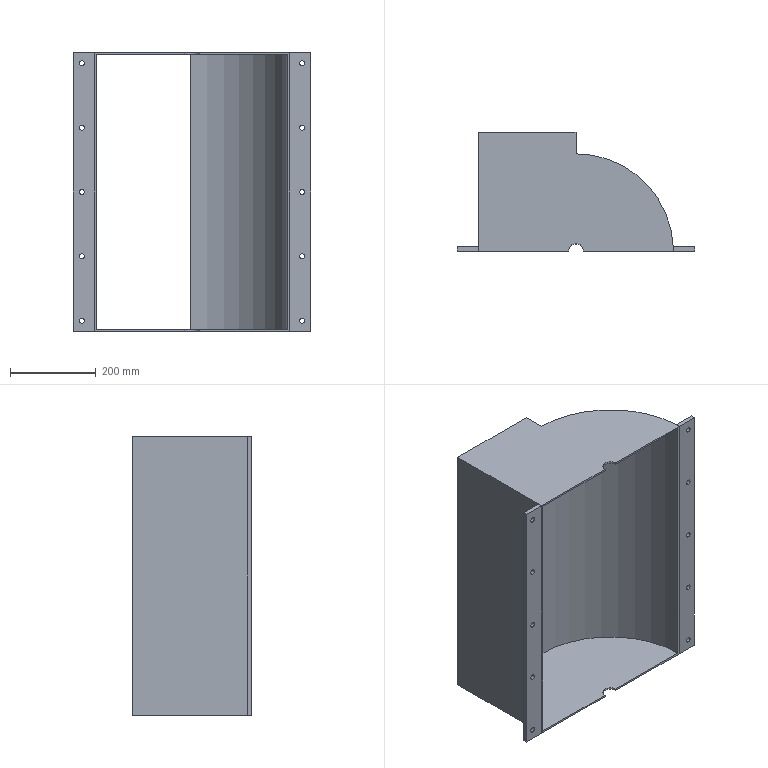Part | SolidWorks | features ICE 5, LPattern 2, Extrusion 1 | 3 solids | 50 faces | box 554 x 277 x 650 mm | volume 3183644 mm3 | cylinder 26 | plane 24 | commonest cylinder face diameters 12 x20 454 x3 35 x2 446 x1
STEP:
#1=CARTESIAN_POINT('',(-257.,10.,294.));
#2=VERTEX_POINT('',#1);
#3=CARTESIAN_POINT('',(-257.,10.,306.));
#4=VERTEX_POINT('',#3);
#5=CARTESIAN_POINT('',(-257.,10.,300.));
#6=DIRECTION('',(0.,1.,0.));
#7=DIRECTION('',(0.,0.,1.));
#8=AXIS2_PLACEMENT_3D('',#5,#6,#7);
#9=CIRCLE('',#8,6.);
#10=EDGE_CURVE('',#2,#4,#9,.T.);
#11=ORIENTED_EDGE('',*,*,#10,.T.);
#12=CARTESIAN_POINT('',(-257.,0.,306.));
#13=VERTEX_POINT('',#12);
#14=CARTESIAN_POINT('',(-257.,377.,306.));
#15=DIRECTION('',(0.,-1.,0.));
#16=VECTOR('',#15,1000.);
#17=LINE('',#14,#16);
#18=EDGE_CURVE('',#4,#13,#17,.T.);
#19=ORIENTED_EDGE('',*,*,#18,.T.);
#20=CARTESIAN_POINT('',(-257.,0.,294.));
#21=VERTEX_POINT('',#20);
#22=CARTESIAN_POINT('',(-257.,0.,300.));
#23=DIRECTION('',(0.,1.,0.));
#24=DIRECTION('',(0.,0.,1.));
#25=AXIS2_PLACEMENT_3D('',#22,#23,#24);
#26=CIRCLE('',#25,6.);
#27=EDGE_CURVE('',#21,#13,#26,.T.);
#28=ORIENTED_EDGE('',*,*,#27,.F.);
#29=CARTESIAN_POINT('',(-257.,377.,294.));
#30=DIRECTION('',(0.,-1.,0.));
#31=VECTOR('',#30,1000.);
#32=LINE('',#29,#31);
#33=EDGE_CURVE('',#2,#21,#32,.T.);
#34=ORIENTED_EDGE('',*,*,#33,.F.);
#35=EDGE_LOOP('',(#11,#19,#28,#34));
#36=FACE_OUTER_BOUND('',#35,.T.);
#37=CARTESIAN_POINT('',(-257.,377.,300.));
#38=DIRECTION('',(0.,-1.,0.));
#39=DIRECTION('',(0.,0.,-1.));
#40=AXIS2_PLACEMENT_3D('',#37,#38,#39);
#41=CYLINDRICAL_SURFACE('',#40,6.);
#42=ADVANCED_FACE('',(#36),#41,.F.);
#43=CARTESIAN_POINT('',(-257.,10.,144.));
#44=VERTEX_POINT('',#43);
#45=CARTESIAN_POINT('',(-257.,10.,156.));
#46=VERTEX_POINT('',#45);
#47=CARTESIAN_POINT('',(-257.,10.,150.));
#48=DIRECTION('',(0.,1.,0.));
#49=DIRECTION('',(0.,0.,1.));
#50=AXIS2_PLACEMENT_3D('',#47,#48,#49);
#51=CIRCLE('',#50,6.);
#52=EDGE_CURVE('',#44,#46,#51,.T.);
#53=ORIENTED_EDGE('',*,*,#52,.T.);
#54=CARTESIAN_POINT('',(-257.,0.,156.));
#55=VERTEX_POINT('',#54);
#56=CARTESIAN_POINT('',(-257.,377.,156.));
#57=DIRECTION('',(0.,-1.,0.));
#58=VECTOR('',#57,1000.);
#59=LINE('',#56,#58);
#60=EDGE_CURVE('',#46,#55,#59,.T.);
#61=ORIENTED_EDGE('',*,*,#60,.T.);
#62=CARTESIAN_POINT('',(-257.,0.,144.));
#63=VERTEX_POINT('',#62);
#64=CARTESIAN_POINT('',(-257.,0.,150.));
#65=DIRECTION('',(0.,1.,0.));
#66=DIRECTION('',(0.,0.,1.));
#67=AXIS2_PLACEMENT_3D('',#64,#65,#66);
#68=CIRCLE('',#67,6.);
#69=EDGE_CURVE('',#63,#55,#68,.T.);
#70=ORIENTED_EDGE('',*,*,#69,.F.);
#71=CARTESIAN_POINT('',(-257.,377.,144.));
#72=DIRECTION('',(0.,-1.,0.));
#73=VECTOR('',#72,1000.);
#74=LINE('',#71,#73);
#75=EDGE_CURVE('',#44,#63,#74,.T.);
#76=ORIENTED_EDGE('',*,*,#75,.F.);
#77=EDGE_LOOP('',(#53,#61,#70,#76));
#78=FACE_OUTER_BOUND('',#77,.T.);
#79=CARTESIAN_POINT('',(-257.,377.,150.));
#80=DIRECTION('',(0.,-1.,0.));
#81=DIRECTION('',(0.,0.,-1.));
#82=AXIS2_PLACEMENT_3D('',#79,#80,#81);
#83=CYLINDRICAL_SURFACE('',#82,6.);
#84=ADVANCED_FACE('',(#78),#83,.F.);
#85=CARTESIAN_POINT('',(-257.,10.,-306.));
#86=VERTEX_POINT('',#85);
#87=CARTESIAN_POINT('',(-257.,10.,-294.));
#88=VERTEX_POINT('',#87);
#89=CARTESIAN_POINT('',(-257.,10.,-300.));
#90=DIRECTION('',(0.,1.,0.));
#91=DIRECTION('',(0.,0.,1.));
#92=AXIS2_PLACEMENT_3D('',#89,#90,#91);
#93=CIRCLE('',#92,6.);
#94=EDGE_CURVE('',#86,#88,#93,.T.);
#95=ORIENTED_EDGE('',*,*,#94,.T.);
#96=CARTESIAN_POINT('',(-257.,0.,-294.));
#97=VERTEX_POINT('',#96);
#98=CARTESIAN_POINT('',(-257.,377.,-294.));
#99=DIRECTION('',(0.,-1.,0.));
#100=VECTOR('',#99,1000.);
#101=LINE('',#98,#100);
#102=EDGE_CURVE('',#88,#97,#101,.T.);
#103=ORIENTED_EDGE('',*,*,#102,.T.);
#104=CARTESIAN_POINT('',(-257.,0.,-306.));
#105=VERTEX_POINT('',#104);
#106=CARTESIAN_POINT('',(-257.,0.,-300.));
#107=DIRECTION('',(0.,1.,0.));
#108=DIRECTION('',(0.,0.,1.));
#109=AXIS2_PLACEMENT_3D('',#106,#107,#108);
#110=CIRCLE('',#109,6.);
#111=EDGE_CURVE('',#105,#97,#110,.T.);
#112=ORIENTED_EDGE('',*,*,#111,.F.);
#113=CARTESIAN_POINT('',(-257.,377.,-306.));
#114=DIRECTION('',(0.,-1.,0.));
#115=VECTOR('',#114,1000.);
#116=LINE('',#113,#115);
#117=EDGE_CURVE('',#86,#105,#116,.T.);
#118=ORIENTED_EDGE('',*,*,#117,.F.);
#119=EDGE_LOOP('',(#95,#103,#112,#118));
#120=FACE_OUTER_BOUND('',#119,.T.);
#121=CARTESIAN_POINT('',(-257.,377.,-300.));
#122=DIRECTION('',(0.,-1.,0.));
#123=DIRECTION('',(0.,0.,-1.));
#124=AXIS2_PLACEMENT_3D('',#121,#122,#123);
#125=CYLINDRICAL_SURFACE('',#124,6.);
#126=ADVANCED_FACE('',(#120),#125,.F.);
#127=CARTESIAN_POINT('',(-257.,10.,-156.));
#128=VERTEX_POINT('',#127);
#129=CARTESIAN_POINT('',(-257.,10.,-144.));
#130=VERTEX_POINT('',#129);
#131=CARTESIAN_POINT('',(-257.,10.,-150.));
#132=DIRECTION('',(0.,1.,0.));
#133=DIRECTION('',(0.,0.,1.));
#134=AXIS2_PLACEMENT_3D('',#131,#132,#133);
#135=CIRCLE('',#134,6.);
#136=EDGE_CURVE('',#128,#130,#135,.T.);
#137=ORIENTED_EDGE('',*,*,#136,.T.);
#138=CARTESIAN_POINT('',(-257.,0.,-144.));
#139=VERTEX_POINT('',#138);
#140=CARTESIAN_POINT('',(-257.,377.,-144.));
#141=DIRECTION('',(0.,-1.,0.));
#142=VECTOR('',#141,1000.);
#143=LINE('',#140,#142);
#144=EDGE_CURVE('',#130,#139,#143,.T.);
#145=ORIENTED_EDGE('',*,*,#144,.T.);
#146=CARTESIAN_POINT('',(-257.,0.,-156.));
#147=VERTEX_POINT('',#146);
#148=CARTESIAN_POINT('',(-257.,0.,-150.));
#149=DIRECTION('',(0.,1.,0.));
#150=DIRECTION('',(0.,0.,1.));
#151=AXIS2_PLACEMENT_3D('',#148,#149,#150);
#152=CIRCLE('',#151,6.);
#153=EDGE_CURVE('',#147,#139,#152,.T.);
#154=ORIENTED_EDGE('',*,*,#153,.F.);
#155=CARTESIAN_POINT('',(-257.,377.,-156.));
#156=DIRECTION('',(0.,-1.,0.));
#157=VECTOR('',#156,1000.);
#158=LINE('',#155,#157);
#159=EDGE_CURVE('',#128,#147,#158,.T.);
#160=ORIENTED_EDGE('',*,*,#159,.F.);
#161=EDGE_LOOP('',(#137,#145,#154,#160));
#162=FACE_OUTER_BOUND('',#161,.T.);
#163=CARTESIAN_POINT('',(-257.,377.,-150.));
#164=DIRECTION('',(0.,-1.,0.));
#165=DIRECTION('',(0.,0.,-1.));
#166=AXIS2_PLACEMENT_3D('',#163,#164,#165);
#167=CYLINDRICAL_SURFACE('',#166,6.);
#168=ADVANCED_FACE('',(#162),#167,.F.);
#169=CARTESIAN_POINT('',(-257.,10.,-6.));
#170=VERTEX_POINT('',#169);
#171=CARTESIAN_POINT('',(-257.,10.,6.));
#172=VERTEX_POINT('',#171);
#173=CARTESIAN_POINT('',(-257.,10.,0.));
#174=DIRECTION('',(0.,1.,0.));
#175=DIRECTION('',(0.,0.,1.));
#176=AXIS2_PLACEMENT_3D('',#173,#174,#175);
#177=CIRCLE('',#176,6.);
#178=EDGE_CURVE('',#170,#172,#177,.T.);
#179=ORIENTED_EDGE('',*,*,#178,.T.);
#180=CARTESIAN_POINT('',(-257.,0.,6.));
#181=VERTEX_POINT('',#180);
#182=CARTESIAN_POINT('',(-257.,377.,6.));
#183=DIRECTION('',(0.,-1.,0.));
#184=VECTOR('',#183,1000.);
#185=LINE('',#182,#184);
#186=EDGE_CURVE('',#172,#181,#185,.T.);
#187=ORIENTED_EDGE('',*,*,#186,.T.);
#188=CARTESIAN_POINT('',(-257.,0.,-6.));
#189=VERTEX_POINT('',#188);
#190=CARTESIAN_POINT('',(-257.,0.,0.));
#191=DIRECTION('',(0.,1.,0.));
#192=DIRECTION('',(0.,0.,1.));
#193=AXIS2_PLACEMENT_3D('',#190,#191,#192);
#194=CIRCLE('',#193,6.);
#195=EDGE_CURVE('',#189,#181,#194,.T.);
#196=ORIENTED_EDGE('',*,*,#195,.F.);
#197=CARTESIAN_POINT('',(-257.,377.,-6.));
#198=DIRECTION('',(0.,-1.,0.));
#199=VECTOR('',#198,1000.);
#200=LINE('',#197,#199);
#201=EDGE_CURVE('',#170,#189,#200,.T.);
#202=ORIENTED_EDGE('',*,*,#201,.F.);
#203=EDGE_LOOP('',(#179,#187,#196,#202));
#204=FACE_OUTER_BOUND('',#203,.T.);
#205=CARTESIAN_POINT('',(-257.,377.,0.));
#206=DIRECTION('',(0.,-1.,0.));
#207=DIRECTION('',(0.,0.,-1.));
#208=AXIS2_PLACEMENT_3D('',#205,#206,#207);
#209=CYLINDRICAL_SURFACE('',#208,6.);
#210=ADVANCED_FACE('',(#204),#209,.F.);
#211=ORIENTED_EDGE('',*,*,#10,.F.);
#212=CARTESIAN_POINT('',(-257.,10.,300.));
#213=DIRECTION('',(0.,1.,0.));
#214=DIRECTION('',(0.,0.,1.));
#215=AXIS2_PLACEMENT_3D('',#212,#213,#214);
#216=CIRCLE('',#215,6.);
#217=EDGE_CURVE('',#4,#2,#216,.T.);
#218=ORIENTED_EDGE('',*,*,#217,.F.);
#219=EDGE_LOOP('',(#211,#218));
#220=FACE_BOUND('',#219,.T.);
#221=ORIENTED_EDGE('',*,*,#52,.F.);
#222=CARTESIAN_POINT('',(-257.,10.,150.));
#223=DIRECTION('',(0.,1.,0.));
#224=DIRECTION('',(0.,0.,1.));
#225=AXIS2_PLACEMENT_3D('',#222,#223,#224);
#226=CIRCLE('',#225,6.);
#227=EDGE_CURVE('',#46,#44,#226,.T.);
#228=ORIENTED_EDGE('',*,*,#227,.F.);
#229=EDGE_LOOP('',(#221,#228));
#230=FACE_BOUND('',#229,.T.);
#231=ORIENTED_EDGE('',*,*,#94,.F.);
#232=CARTESIAN_POINT('',(-257.,10.,-300.));
#233=DIRECTION('',(0.,1.,0.));
#234=DIRECTION('',(0.,0.,1.));
#235=AXIS2_PLACEMENT_3D('',#232,#233,#234);
#236=CIRCLE('',#235,6.);
#237=EDGE_CURVE('',#88,#86,#236,.T.);
#238=ORIENTED_EDGE('',*,*,#237,.F.);
#239=EDGE_LOOP('',(#231,#238));
#240=FACE_BOUND('',#239,.T.);
#241=ORIENTED_EDGE('',*,*,#136,.F.);
#242=CARTESIAN_POINT('',(-257.,10.,-150.));
#243=DIRECTION('',(0.,1.,0.));
#244=DIRECTION('',(0.,0.,1.));
#245=AXIS2_PLACEMENT_3D('',#242,#243,#244);
#246=CIRCLE('',#245,6.);
#247=EDGE_CURVE('',#130,#128,#246,.T.);
#248=ORIENTED_EDGE('',*,*,#247,.F.);
#249=EDGE_LOOP('',(#241,#248));
#250=FACE_BOUND('',#249,.T.);
#251=ORIENTED_EDGE('',*,*,#178,.F.);
#252=CARTESIAN_POINT('',(-257.,10.,0.));
#253=DIRECTION('',(0.,1.,0.));
#254=DIRECTION('',(0.,0.,1.));
#255=AXIS2_PLACEMENT_3D('',#252,#253,#254);
#256=CIRCLE('',#255,6.);
#257=EDGE_CURVE('',#172,#170,#256,.T.);
#258=ORIENTED_EDGE('',*,*,#257,.F.);
#259=EDGE_LOOP('',(#251,#258));
#260=FACE_BOUND('',#259,.T.);
#261=CARTESIAN_POINT('',(-277.,10.,-325.));
#262=VERTEX_POINT('',#261);
#263=CARTESIAN_POINT('',(-227.,10.,-325.));
#264=VERTEX_POINT('',#263);
#265=CARTESIAN_POINT('',(0.,10.,-325.));
#266=DIRECTION('',(1.,0.,0.));
#267=VECTOR('',#266,1000.);
#268=LINE('',#265,#267);
#269=EDGE_CURVE('',#262,#264,#268,.T.);
#270=ORIENTED_EDGE('',*,*,#269,.F.);
#271=CARTESIAN_POINT('',(-277.,10.,325.));
#272=VERTEX_POINT('',#271);
#273=CARTESIAN_POINT('',(-277.,10.,325.));
#274=DIRECTION('',(0.,0.,-1.));
#275=VECTOR('',#274,1000.);
#276=LINE('',#273,#275);
#277=EDGE_CURVE('',#272,#262,#276,.T.);
#278=ORIENTED_EDGE('',*,*,#277,.F.);
#279=CARTESIAN_POINT('',(-227.,10.,325.));
#280=VERTEX_POINT('',#279);
#281=CARTESIAN_POINT('',(0.,10.,325.));
#282=DIRECTION('',(1.,0.,0.));
#283=VECTOR('',#282,1000.);
#284=LINE('',#281,#283);
#285=EDGE_CURVE('',#272,#280,#284,.T.);
#286=ORIENTED_EDGE('',*,*,#285,.T.);
#287=CARTESIAN_POINT('',(-227.,10.,325.));
#288=DIRECTION('',(0.,0.,-1.));
#289=VECTOR('',#288,1000.);
#290=LINE('',#287,#289);
#291=EDGE_CURVE('',#280,#264,#290,.T.);
#292=ORIENTED_EDGE('',*,*,#291,.T.);
#293=EDGE_LOOP('',(#270,#278,#286,#292));
#294=FACE_OUTER_BOUND('',#293,.T.);
#295=CARTESIAN_POINT('',(0.,10.,325.));
#296=DIRECTION('',(0.,1.,0.));
#297=DIRECTION('',(0.,0.,1.));
#298=AXIS2_PLACEMENT_3D('',#295,#296,#297);
#299=PLANE('',#298);
#300=ADVANCED_FACE('',(#220,#230,#240,#250,#260,#294),#299,.T.);
#301=CARTESIAN_POINT('',(-277.,0.,-325.));
#302=VERTEX_POINT('',#301);
#303=CARTESIAN_POINT('',(-277.,0.,-325.));
#304=DIRECTION('',(0.,1.,0.));
#305=VECTOR('',#304,1000.);
#306=LINE('',#303,#305);
#307=EDGE_CURVE('',#302,#262,#306,.T.);
#308=ORIENTED_EDGE('',*,*,#307,.F.);
#309=CARTESIAN_POINT('',(-277.,0.,325.));
#310=VERTEX_POINT('',#309);
#311=CARTESIAN_POINT('',(-277.,0.,325.));
#312=DIRECTION('',(0.,0.,-1.));
#313=VECTOR('',#312,1000.);
#314=LINE('',#311,#313);
#315=EDGE_CURVE('',#310,#302,#314,.T.);
#316=ORIENTED_EDGE('',*,*,#315,.F.);
#317=CARTESIAN_POINT('',(-277.,0.,325.));
#318=DIRECTION('',(0.,1.,0.));
#319=VECTOR('',#318,1000.);
#320=LINE('',#317,#319);
#321=EDGE_CURVE('',#310,#272,#320,.T.);
#322=ORIENTED_EDGE('',*,*,#321,.T.);
#323=ORIENTED_EDGE('',*,*,#277,.T.);
#324=EDGE_LOOP('',(#308,#316,#322,#323));
#325=FACE_OUTER_BOUND('',#324,.T.);
#326=CARTESIAN_POINT('',(-277.,0.,325.));
#327=DIRECTION('',(-1.,0.,0.));
#328=DIRECTION('',(0.,0.,1.));
#329=AXIS2_PLACEMENT_3D('',#326,#327,#328);
#330=PLANE('',#329);
#331=ADVANCED_FACE('',(#325),#330,.T.);
#332=ORIENTED_EDGE('',*,*,#27,.T.);
#333=CARTESIAN_POINT('',(-257.,0.,300.));
#334=DIRECTION('',(0.,1.,0.));
#335=DIRECTION('',(0.,0.,1.));
#336=AXIS2_PLACEMENT_3D('',#333,#334,#335);
#337=CIRCLE('',#336,6.);
#338=EDGE_CURVE('',#13,#21,#337,.T.);
#339=ORIENTED_EDGE('',*,*,#338,.T.);
#340=EDGE_LOOP('',(#332,#339));
#341=FACE_BOUND('',#340,.T.);
#342=ORIENTED_EDGE('',*,*,#69,.T.);
#343=CARTESIAN_POINT('',(-257.,0.,150.));
#344=DIRECTION('',(0.,1.,0.));
#345=DIRECTION('',(0.,0.,1.));
#346=AXIS2_PLACEMENT_3D('',#343,#344,#345);
#347=CIRCLE('',#346,6.);
#348=EDGE_CURVE('',#55,#63,#347,.T.);
#349=ORIENTED_EDGE('',*,*,#348,.T.);
#350=EDGE_LOOP('',(#342,#349));
#351=FACE_BOUND('',#350,.T.);
#352=ORIENTED_EDGE('',*,*,#111,.T.);
#353=CARTESIAN_POINT('',(-257.,0.,-300.));
#354=DIRECTION('',(0.,1.,0.));
#355=DIRECTION('',(0.,0.,1.));
#356=AXIS2_PLACEMENT_3D('',#353,#354,#355);
#357=CIRCLE('',#356,6.);
#358=EDGE_CURVE('',#97,#105,#357,.T.);
#359=ORIENTED_EDGE('',*,*,#358,.T.);
#360=EDGE_LOOP('',(#352,#359));
#361=FACE_BOUND('',#360,.T.);
#362=ORIENTED_EDGE('',*,*,#153,.T.);
#363=CARTESIAN_POINT('',(-257.,0.,-150.));
#364=DIRECTION('',(0.,1.,0.));
#365=DIRECTION('',(0.,0.,1.));
#366=AXIS2_PLACEMENT_3D('',#363,#364,#365);
#367=CIRCLE('',#366,6.);
#368=EDGE_CURVE('',#139,#147,#367,.T.);
#369=ORIENTED_EDGE('',*,*,#368,.T.);
#370=EDGE_LOOP('',(#362,#369));
#371=FACE_BOUND('',#370,.T.);
#372=ORIENTED_EDGE('',*,*,#195,.T.);
#373=CARTESIAN_POINT('',(-257.,0.,0.));
#374=DIRECTION('',(0.,1.,0.));
#375=DIRECTION('',(0.,0.,1.));
#376=AXIS2_PLACEMENT_3D('',#373,#374,#375);
#377=CIRCLE('',#376,6.);
#378=EDGE_CURVE('',#181,#189,#377,.T.);
#379=ORIENTED_EDGE('',*,*,#378,.T.);
#380=EDGE_LOOP('',(#372,#379));
#381=FACE_BOUND('',#380,.T.);
#382=CARTESIAN_POINT('',(-227.,0.,-325.));
#383=VERTEX_POINT('',#382);
#384=CARTESIAN_POINT('',(0.,0.,-325.));
#385=DIRECTION('',(1.,0.,0.));
#386=VECTOR('',#385,1000.);
#387=LINE('',#384,#386);
#388=EDGE_CURVE('',#302,#383,#387,.T.);
#389=ORIENTED_EDGE('',*,*,#388,.T.);
#390=CARTESIAN_POINT('',(-227.,0.,325.));
#391=VERTEX_POINT('',#390);
#392=CARTESIAN_POINT('',(-227.,0.,325.));
#393=DIRECTION('',(0.,0.,-1.));
#394=VECTOR('',#393,1000.);
#395=LINE('',#392,#394);
#396=EDGE_CURVE('',#391,#383,#395,.T.);
#397=ORIENTED_EDGE('',*,*,#396,.F.);
#398=CARTESIAN_POINT('',(0.,0.,325.));
#399=DIRECTION('',(1.,0.,0.));
#400=VECTOR('',#399,1000.);
#401=LINE('',#398,#400);
#402=EDGE_CURVE('',#310,#391,#401,.T.);
#403=ORIENTED_EDGE('',*,*,#402,.F.);
#404=ORIENTED_EDGE('',*,*,#315,.T.);
#405=EDGE_LOOP('',(#389,#397,#403,#404));
#406=FACE_OUTER_BOUND('',#405,.T.);
#407=CARTESIAN_POINT('',(0.,0.,325.));
#408=DIRECTION('',(0.,1.,0.));
#409=DIRECTION('',(0.,0.,1.));
#410=AXIS2_PLACEMENT_3D('',#407,#408,#409);
#411=PLANE('',#410);
#412=ADVANCED_FACE('',(#341,#351,#361,#371,#381,#406),#411,.F.);
#413=CARTESIAN_POINT('',(-227.,0.,-325.));
#414=DIRECTION('',(0.,1.,0.));
#415=VECTOR('',#414,1000.);
#416=LINE('',#413,#415);
#417=EDGE_CURVE('',#383,#264,#416,.T.);
#418=ORIENTED_EDGE('',*,*,#417,.T.);
#419=ORIENTED_EDGE('',*,*,#291,.F.);
#420=CARTESIAN_POINT('',(-227.,0.,325.));
#421=DIRECTION('',(0.,1.,0.));
#422=VECTOR('',#421,1000.);
#423=LINE('',#420,#422);
#424=EDGE_CURVE('',#391,#280,#423,.T.);
#425=ORIENTED_EDGE('',*,*,#424,.F.);
#426=ORIENTED_EDGE('',*,*,#396,.T.);
#427=EDGE_LOOP('',(#418,#419,#425,#426));
#428=FACE_OUTER_BOUND('',#427,.T.);
#429=CARTESIAN_POINT('',(-227.,0.,325.));
#430=DIRECTION('',(-1.,0.,0.));
#431=DIRECTION('',(0.,0.,1.));
#432=AXIS2_PLACEMENT_3D('',#429,#430,#431);
#433=PLANE('',#432);
#434=ADVANCED_FACE('',(#428),#433,.F.);
#435=ORIENTED_EDGE('',*,*,#285,.F.);
#436=ORIENTED_EDGE('',*,*,#321,.F.);
#437=ORIENTED_EDGE('',*,*,#402,.T.);
#438=ORIENTED_EDGE('',*,*,#424,.T.);
#439=EDGE_LOOP('',(#435,#436,#437,#438));
#440=FACE_OUTER_BOUND('',#439,.T.);
#441=CARTESIAN_POINT('',(0.,0.,325.));
#442=DIRECTION('',(0.,0.,1.));
#443=DIRECTION('',(1.,0.,0.));
#444=AXIS2_PLACEMENT_3D('',#441,#442,#443);
#445=PLANE('',#444);
#446=ADVANCED_FACE('',(#440),#445,.T.);
#447=ORIENTED_EDGE('',*,*,#269,.T.);
#448=ORIENTED_EDGE('',*,*,#417,.F.);
#449=ORIENTED_EDGE('',*,*,#388,.F.);
#450=ORIENTED_EDGE('',*,*,#307,.T.);
#451=EDGE_LOOP('',(#447,#448,#449,#450));
#452=FACE_OUTER_BOUND('',#451,.T.);
#453=CARTESIAN_POINT('',(0.,0.,-325.));
#454=DIRECTION('',(0.,0.,1.));
#455=DIRECTION('',(1.,0.,0.));
#456=AXIS2_PLACEMENT_3D('',#453,#454,#455);
#457=PLANE('',#456);
#458=ADVANCED_FACE('',(#452),#457,.F.);
#459=ORIENTED_EDGE('',*,*,#186,.F.);
#460=ORIENTED_EDGE('',*,*,#257,.T.);
#461=ORIENTED_EDGE('',*,*,#201,.T.);
#462=ORIENTED_EDGE('',*,*,#378,.F.);
#463=EDGE_LOOP('',(#459,#460,#461,#462));
#464=FACE_OUTER_BOUND('',#463,.T.);
#465=CARTESIAN_POINT('',(-257.,377.,0.));
#466=DIRECTION('',(0.,-1.,0.));
#467=DIRECTION('',(0.,0.,-1.));
#468=AXIS2_PLACEMENT_3D('',#465,#466,#467);
#469=CYLINDRICAL_SURFACE('',#468,6.);
#470=ADVANCED_FACE('',(#464),#469,.F.);
#471=ORIENTED_EDGE('',*,*,#144,.F.);
#472=ORIENTED_EDGE('',*,*,#247,.T.);
#473=ORIENTED_EDGE('',*,*,#159,.T.);
#474=ORIENTED_EDGE('',*,*,#368,.F.);
#475=EDGE_LOOP('',(#471,#472,#473,#474));
#476=FACE_OUTER_BOUND('',#475,.T.);
#477=CARTESIAN_POINT('',(-257.,377.,-150.));
#478=DIRECTION('',(0.,-1.,0.));
#479=DIRECTION('',(0.,0.,-1.));
#480=AXIS2_PLACEMENT_3D('',#477,#478,#479);
#481=CYLINDRICAL_SURFACE('',#480,6.);
#482=ADVANCED_FACE('',(#476),#481,.F.);
#483=ORIENTED_EDGE('',*,*,#102,.F.);
#484=ORIENTED_EDGE('',*,*,#237,.T.);
#485=ORIENTED_EDGE('',*,*,#117,.T.);
#486=ORIENTED_EDGE('',*,*,#358,.F.);
#487=EDGE_LOOP('',(#483,#484,#485,#486));
#488=FACE_OUTER_BOUND('',#487,.T.);
#489=CARTESIAN_POINT('',(-257.,377.,-300.));
#490=DIRECTION('',(0.,-1.,0.));
#491=DIRECTION('',(0.,0.,-1.));
#492=AXIS2_PLACEMENT_3D('',#489,#490,#491);
#493=CYLINDRICAL_SURFACE('',#492,6.);
#494=ADVANCED_FACE('',(#488),#493,.F.);
#495=ORIENTED_EDGE('',*,*,#60,.F.);
#496=ORIENTED_EDGE('',*,*,#227,.T.);
#497=ORIENTED_EDGE('',*,*,#75,.T.);
#498=ORIENTED_EDGE('',*,*,#348,.F.);
#499=EDGE_LOOP('',(#495,#496,#497,#498));
#500=FACE_OUTER_BOUND('',#499,.T.);
#501=CARTESIAN_POINT('',(-257.,377.,150.));
#502=DIRECTION('',(0.,-1.,0.));
#503=DIRECTION('',(0.,0.,-1.));
#504=AXIS2_PLACEMENT_3D('',#501,#502,#503);
#505=CYLINDRICAL_SURFACE('',#504,6.);
#506=ADVANCED_FACE('',(#500),#505,.F.);
#507=ORIENTED_EDGE('',*,*,#18,.F.);
#508=ORIENTED_EDGE('',*,*,#217,.T.);
#509=ORIENTED_EDGE('',*,*,#33,.T.);
#510=ORIENTED_EDGE('',*,*,#338,.F.);
#511=EDGE_LOOP('',(#507,#508,#509,#510));
#512=FACE_OUTER_BOUND('',#511,.T.);
#513=CARTESIAN_POINT('',(-257.,377.,300.));
#514=DIRECTION('',(0.,-1.,0.));
#515=DIRECTION('',(0.,0.,-1.));
#516=AXIS2_PLACEMENT_3D('',#513,#514,#515);
#517=CYLINDRICAL_SURFACE('',#516,6.);
#518=ADVANCED_FACE('',(#512),#517,.F.);
#519=CLOSED_SHELL('',(#42,#84,#126,#168,#210,#300,#331,#412,#434,#446,#458,#470,#482,#494,#506,#518));
#520=MANIFOLD_SOLID_BREP('',#519);
#521=CARTESIAN_POINT('',(257.,10.,306.));
#522=VERTEX_POINT('',#521);
#523=CARTESIAN_POINT('',(257.,10.,294.));
#524=VERTEX_POINT('',#523);
#525=CARTESIAN_POINT('',(257.,10.,300.));
#526=DIRECTION('',(0.,-1.,0.));
#527=DIRECTION('',(1.,0.,0.));
#528=AXIS2_PLACEMENT_3D('',#525,#526,#527);
#529=CIRCLE('',#528,6.);
#530=EDGE_CURVE('',#522,#524,#529,.T.);
#531=ORIENTED_EDGE('',*,*,#530,.F.);
#532=CARTESIAN_POINT('',(257.,0.,306.));
#533=VERTEX_POINT('',#532);
#534=CARTESIAN_POINT('',(257.,377.,306.));
#535=DIRECTION('',(0.,-1.,0.));
#536=VECTOR('',#535,1000.);
#537=LINE('',#534,#536);
#538=EDGE_CURVE('',#522,#533,#537,.T.);
#539=ORIENTED_EDGE('',*,*,#538,.T.);
#540=CARTESIAN_POINT('',(257.,0.,294.));
#541=VERTEX_POINT('',#540);
#542=CARTESIAN_POINT('',(257.,0.,300.));
#543=DIRECTION('',(0.,-1.,0.));
#544=DIRECTION('',(1.,0.,0.));
#545=AXIS2_PLACEMENT_3D('',#542,#543,#544);
#546=CIRCLE('',#545,6.);
#547=EDGE_CURVE('',#533,#541,#546,.T.);
#548=ORIENTED_EDGE('',*,*,#547,.T.);
#549=CARTESIAN_POINT('',(257.,377.,294.));
#550=DIRECTION('',(0.,-1.,0.));
#551=VECTOR('',#550,1000.);
#552=LINE('',#549,#551);
#553=EDGE_CURVE('',#524,#541,#552,.T.);
#554=ORIENTED_EDGE('',*,*,#553,.F.);
#555=EDGE_LOOP('',(#531,#539,#548,#554));
#556=FACE_OUTER_BOUND('',#555,.T.);
#557=CARTESIAN_POINT('',(257.,377.,300.));
#558=DIRECTION('',(0.,-1.,0.));
#559=DIRECTION('',(0.,0.,-1.));
#560=AXIS2_PLACEMENT_3D('',#557,#558,#559);
#561=CYLINDRICAL_SURFACE('',#560,6.);
#562=ADVANCED_FACE('',(#556),#561,.F.);
#563=CARTESIAN_POINT('',(257.,10.,156.));
#564=VERTEX_POINT('',#563);
#565=CARTESIAN_POINT('',(257.,10.,144.));
#566=VERTEX_POINT('',#565);
#567=CARTESIAN_POINT('',(257.,10.,150.));
#568=DIRECTION('',(0.,-1.,0.));
#569=DIRECTION('',(1.,0.,0.));
#570=AXIS2_PLACEMENT_3D('',#567,#568,#569);
#571=CIRCLE('',#570,6.);
#572=EDGE_CURVE('',#564,#566,#571,.T.);
#573=ORIENTED_EDGE('',*,*,#572,.F.);
#574=CARTESIAN_POINT('',(257.,0.,156.));
#575=VERTEX_POINT('',#574);
#576=CARTESIAN_POINT('',(257.,377.,156.));
#577=DIRECTION('',(0.,-1.,0.));
#578=VECTOR('',#577,1000.);
#579=LINE('',#576,#578);
#580=EDGE_CURVE('',#564,#575,#579,.T.);
#581=ORIENTED_EDGE('',*,*,#580,.T.);
#582=CARTESIAN_POINT('',(257.,0.,144.));
#583=VERTEX_POINT('',#582);
#584=CARTESIAN_POINT('',(257.,0.,150.));
#585=DIRECTION('',(0.,-1.,0.));
#586=DIRECTION('',(1.,0.,0.));
#587=AXIS2_PLACEMENT_3D('',#584,#585,#586);
#588=CIRCLE('',#587,6.);
#589=EDGE_CURVE('',#575,#583,#588,.T.);
#590=ORIENTED_EDGE('',*,*,#589,.T.);
#591=CARTESIAN_POINT('',(257.,377.,144.));
#592=DIRECTION('',(0.,-1.,0.));
#593=VECTOR('',#592,1000.);
#594=LINE('',#591,#593);
#595=EDGE_CURVE('',#566,#583,#594,.T.);
#596=ORIENTED_EDGE('',*,*,#595,.F.);
#597=EDGE_LOOP('',(#573,#581,#590,#596));
#598=FACE_OUTER_BOUND('',#597,.T.);
#599=CARTESIAN_POINT('',(257.,377.,150.));
#600=DIRECTION('',(0.,-1.,0.));
#601=DIRECTION('',(0.,0.,-1.));
#602=AXIS2_PLACEMENT_3D('',#599,#600,#601);
#603=CYLINDRICAL_SURFACE('',#602,6.);
#604=ADVANCED_FACE('',(#598),#603,.F.);
#605=CARTESIAN_POINT('',(257.,10.,-294.));
#606=VERTEX_POINT('',#605);
#607=CARTESIAN_POINT('',(257.,10.,-306.));
#608=VERTEX_POINT('',#607);
#609=CARTESIAN_POINT('',(257.,10.,-300.));
#610=DIRECTION('',(0.,-1.,0.));
#611=DIRECTION('',(1.,0.,0.));
#612=AXIS2_PLACEMENT_3D('',#609,#610,#611);
#613=CIRCLE('',#612,6.);
#614=EDGE_CURVE('',#606,#608,#613,.T.);
#615=ORIENTED_EDGE('',*,*,#614,.F.);
#616=CARTESIAN_POINT('',(257.,0.,-294.));
#617=VERTEX_POINT('',#616);
#618=CARTESIAN_POINT('',(257.,377.,-294.));
#619=DIRECTION('',(0.,-1.,0.));
#620=VECTOR('',#619,1000.);
#621=LINE('',#618,#620);
#622=EDGE_CURVE('',#606,#617,#621,.T.);
#623=ORIENTED_EDGE('',*,*,#622,.T.);
#624=CARTESIAN_POINT('',(257.,0.,-306.));
#625=VERTEX_POINT('',#624);
#626=CARTESIAN_POINT('',(257.,0.,-300.));
#627=DIRECTION('',(0.,-1.,0.));
#628=DIRECTION('',(1.,0.,0.));
#629=AXIS2_PLACEMENT_3D('',#626,#627,#628);
#630=CIRCLE('',#629,6.);
#631=EDGE_CURVE('',#617,#625,#630,.T.);
#632=ORIENTED_EDGE('',*,*,#631,.T.);
#633=CARTESIAN_POINT('',(257.,377.,-306.));
#634=DIRECTION('',(0.,-1.,0.));
#635=VECTOR('',#634,1000.);
#636=LINE('',#633,#635);
#637=EDGE_CURVE('',#608,#625,#636,.T.);
#638=ORIENTED_EDGE('',*,*,#637,.F.);
#639=EDGE_LOOP('',(#615,#623,#632,#638));
#640=FACE_OUTER_BOUND('',#639,.T.);
#641=CARTESIAN_POINT('',(257.,377.,-300.));
#642=DIRECTION('',(0.,-1.,0.));
#643=DIRECTION('',(0.,0.,-1.));
#644=AXIS2_PLACEMENT_3D('',#641,#642,#643);
#645=CYLINDRICAL_SURFACE('',#644,6.);
#646=ADVANCED_FACE('',(#640),#645,.F.);
#647=CARTESIAN_POINT('',(257.,10.,-144.));
#648=VERTEX_POINT('',#647);
#649=CARTESIAN_POINT('',(257.,10.,-156.));
#650=VERTEX_POINT('',#649);
#651=CARTESIAN_POINT('',(257.,10.,-150.));
#652=DIRECTION('',(0.,-1.,0.));
#653=DIRECTION('',(1.,0.,0.));
#654=AXIS2_PLACEMENT_3D('',#651,#652,#653);
#655=CIRCLE('',#654,6.);
#656=EDGE_CURVE('',#648,#650,#655,.T.);
#657=ORIENTED_EDGE('',*,*,#656,.F.);
#658=CARTESIAN_POINT('',(257.,0.,-144.));
#659=VERTEX_POINT('',#658);
#660=CARTESIAN_POINT('',(257.,377.,-144.));
#661=DIRECTION('',(0.,-1.,0.));
#662=VECTOR('',#661,1000.);
#663=LINE('',#660,#662);
#664=EDGE_CURVE('',#648,#659,#663,.T.);
#665=ORIENTED_EDGE('',*,*,#664,.T.);
#666=CARTESIAN_POINT('',(257.,0.,-156.));
#667=VERTEX_POINT('',#666);
#668=CARTESIAN_POINT('',(257.,0.,-150.));
#669=DIRECTION('',(0.,-1.,0.));
#670=DIRECTION('',(1.,0.,0.));
#671=AXIS2_PLACEMENT_3D('',#668,#669,#670);
#672=CIRCLE('',#671,6.);
#673=EDGE_CURVE('',#659,#667,#672,.T.);
#674=ORIENTED_EDGE('',*,*,#673,.T.);
#675=CARTESIAN_POINT('',(257.,377.,-156.));
#676=DIRECTION('',(0.,-1.,0.));
#677=VECTOR('',#676,1000.);
#678=LINE('',#675,#677);
#679=EDGE_CURVE('',#650,#667,#678,.T.);
#680=ORIENTED_EDGE('',*,*,#679,.F.);
#681=EDGE_LOOP('',(#657,#665,#674,#680));
#682=FACE_OUTER_BOUND('',#681,.T.);
#683=CARTESIAN_POINT('',(257.,377.,-150.));
#684=DIRECTION('',(0.,-1.,0.));
#685=DIRECTION('',(0.,0.,-1.));
#686=AXIS2_PLACEMENT_3D('',#683,#684,#685);
#687=CYLINDRICAL_SURFACE('',#686,6.);
#688=ADVANCED_FACE('',(#682),#687,.F.);
#689=CARTESIAN_POINT('',(257.,10.,6.));
#690=VERTEX_POINT('',#689);
#691=CARTESIAN_POINT('',(257.,10.,-6.));
#692=VERTEX_POINT('',#691);
#693=CARTESIAN_POINT('',(257.,10.,0.));
#694=DIRECTION('',(0.,-1.,0.));
#695=DIRECTION('',(1.,0.,0.));
#696=AXIS2_PLACEMENT_3D('',#693,#694,#695);
#697=CIRCLE('',#696,6.);
#698=EDGE_CURVE('',#690,#692,#697,.T.);
#699=ORIENTED_EDGE('',*,*,#698,.F.);
#700=CARTESIAN_POINT('',(257.,0.,6.));
#701=VERTEX_POINT('',#700);
#702=CARTESIAN_POINT('',(257.,377.,6.));
#703=DIRECTION('',(0.,-1.,0.));
#704=VECTOR('',#703,1000.);
#705=LINE('',#702,#704);
#706=EDGE_CURVE('',#690,#701,#705,.T.);
#707=ORIENTED_EDGE('',*,*,#706,.T.);
#708=CARTESIAN_POINT('',(257.,0.,-6.));
#709=VERTEX_POINT('',#708);
#710=CARTESIAN_POINT('',(257.,0.,0.));
#711=DIRECTION('',(0.,-1.,0.));
#712=DIRECTION('',(1.,0.,0.));
#713=AXIS2_PLACEMENT_3D('',#710,#711,#712);
#714=CIRCLE('',#713,6.);
#715=EDGE_CURVE('',#701,#709,#714,.T.);
#716=ORIENTED_EDGE('',*,*,#715,.T.);
#717=CARTESIAN_POINT('',(257.,377.,-6.));
#718=DIRECTION('',(0.,-1.,0.));
#719=VECTOR('',#718,1000.);
#720=LINE('',#717,#719);
#721=EDGE_CURVE('',#692,#709,#720,.T.);
#722=ORIENTED_EDGE('',*,*,#721,.F.);
#723=EDGE_LOOP('',(#699,#707,#716,#722));
#724=FACE_OUTER_BOUND('',#723,.T.);
#725=CARTESIAN_POINT('',(257.,377.,0.));
#726=DIRECTION('',(0.,-1.,0.));
#727=DIRECTION('',(0.,0.,-1.));
#728=AXIS2_PLACEMENT_3D('',#725,#726,#727);
#729=CYLINDRICAL_SURFACE('',#728,6.);
#730=ADVANCED_FACE('',(#724),#729,.F.);
#731=CARTESIAN_POINT('',(227.,0.,-325.));
#732=VERTEX_POINT('',#731);
#733=CARTESIAN_POINT('',(226.78,10.,-325.));
#734=VERTEX_POINT('',#733);
#735=CARTESIAN_POINT('',(0.,0.,-325.));
#736=DIRECTION('',(0.,0.,1.));
#737=DIRECTION('',(1.,0.,0.));
#738=AXIS2_PLACEMENT_3D('',#735,#736,#737);
#739=CIRCLE('',#738,227.);
#740=EDGE_CURVE('',#732,#734,#739,.T.);
#741=ORIENTED_EDGE('',*,*,#740,.F.);
#742=CARTESIAN_POINT('',(227.,0.,325.));
#743=VERTEX_POINT('',#742);
#744=CARTESIAN_POINT('',(227.,0.,325.));
#745=DIRECTION('',(0.,0.,-1.));
#746=VECTOR('',#745,1000.);
#747=LINE('',#744,#746);
#748=EDGE_CURVE('',#743,#732,#747,.T.);
#749=ORIENTED_EDGE('',*,*,#748,.F.);
#750=CARTESIAN_POINT('',(226.78,10.,325.));
#751=VERTEX_POINT('',#750);
#752=CARTESIAN_POINT('',(0.,0.,325.));
#753=DIRECTION('',(0.,0.,1.));
#754=DIRECTION('',(1.,0.,0.));
#755=AXIS2_PLACEMENT_3D('',#752,#753,#754);
#756=CIRCLE('',#755,227.);
#757=EDGE_CURVE('',#743,#751,#756,.T.);
#758=ORIENTED_EDGE('',*,*,#757,.T.);
#759=CARTESIAN_POINT('',(226.78,10.,325.));
#760=DIRECTION('',(0.,0.,-1.));
#761=VECTOR('',#760,1000.);
#762=LINE('',#759,#761);
#763=EDGE_CURVE('',#751,#734,#762,.T.);
#764=ORIENTED_EDGE('',*,*,#763,.T.);
#765=EDGE_LOOP('',(#741,#749,#758,#764));
#766=FACE_OUTER_BOUND('',#765,.T.);
#767=CARTESIAN_POINT('',(0.,0.,325.));
#768=DIRECTION('',(0.,0.,-1.));
#769=DIRECTION('',(-1.,0.,0.));
#770=AXIS2_PLACEMENT_3D('',#767,#768,#769);
#771=CYLINDRICAL_SURFACE('',#770,227.);
#772=ADVANCED_FACE('',(#766),#771,.F.);
#773=CARTESIAN_POINT('',(257.,0.,300.));
#774=DIRECTION('',(0.,-1.,0.));
#775=DIRECTION('',(1.,0.,0.));
#776=AXIS2_PLACEMENT_3D('',#773,#774,#775);
#777=CIRCLE('',#776,6.);
#778=EDGE_CURVE('',#541,#533,#777,.T.);
#779=ORIENTED_EDGE('',*,*,#778,.F.);
#780=ORIENTED_EDGE('',*,*,#547,.F.);
#781=EDGE_LOOP('',(#779,#780));
#782=FACE_BOUND('',#781,.T.);
#783=CARTESIAN_POINT('',(257.,0.,150.));
#784=DIRECTION('',(0.,-1.,0.));
#785=DIRECTION('',(1.,0.,0.));
#786=AXIS2_PLACEMENT_3D('',#783,#784,#785);
#787=CIRCLE('',#786,6.);
#788=EDGE_CURVE('',#583,#575,#787,.T.);
#789=ORIENTED_EDGE('',*,*,#788,.F.);
#790=ORIENTED_EDGE('',*,*,#589,.F.);
#791=EDGE_LOOP('',(#789,#790));
#792=FACE_BOUND('',#791,.T.);
#793=CARTESIAN_POINT('',(257.,0.,-300.));
#794=DIRECTION('',(0.,-1.,0.));
#795=DIRECTION('',(1.,0.,0.));
#796=AXIS2_PLACEMENT_3D('',#793,#794,#795);
#797=CIRCLE('',#796,6.);
#798=EDGE_CURVE('',#625,#617,#797,.T.);
#799=ORIENTED_EDGE('',*,*,#798,.F.);
#800=ORIENTED_EDGE('',*,*,#631,.F.);
#801=EDGE_LOOP('',(#799,#800));
#802=FACE_BOUND('',#801,.T.);
#803=CARTESIAN_POINT('',(257.,0.,-150.));
#804=DIRECTION('',(0.,-1.,0.));
#805=DIRECTION('',(1.,0.,0.));
#806=AXIS2_PLACEMENT_3D('',#803,#804,#805);
#807=CIRCLE('',#806,6.);
#808=EDGE_CURVE('',#667,#659,#807,.T.);
#809=ORIENTED_EDGE('',*,*,#808,.F.);
#810=ORIENTED_EDGE('',*,*,#673,.F.);
#811=EDGE_LOOP('',(#809,#810));
#812=FACE_BOUND('',#811,.T.);
#813=CARTESIAN_POINT('',(257.,0.,0.));
#814=DIRECTION('',(0.,-1.,0.));
#815=DIRECTION('',(1.,0.,0.));
#816=AXIS2_PLACEMENT_3D('',#813,#814,#815);
#817=CIRCLE('',#816,6.);
#818=EDGE_CURVE('',#709,#701,#817,.T.);
#819=ORIENTED_EDGE('',*,*,#818,.F.);
#820=ORIENTED_EDGE('',*,*,#715,.F.);
#821=EDGE_LOOP('',(#819,#820));
#822=FACE_BOUND('',#821,.T.);
#823=CARTESIAN_POINT('',(277.,0.,-325.));
#824=VERTEX_POINT('',#823);
#825=CARTESIAN_POINT('',(0.,0.,-325.));
#826=DIRECTION('',(-1.,0.,0.));
#827=VECTOR('',#826,1000.);
#828=LINE('',#825,#827);
#829=EDGE_CURVE('',#824,#732,#828,.T.);
#830=ORIENTED_EDGE('',*,*,#829,.F.);
#831=CARTESIAN_POINT('',(277.,0.,325.));
#832=VERTEX_POINT('',#831);
#833=CARTESIAN_POINT('',(277.,0.,325.));
#834=DIRECTION('',(0.,0.,-1.));
#835=VECTOR('',#834,1000.);
#836=LINE('',#833,#835);
#837=EDGE_CURVE('',#832,#824,#836,.T.);
#838=ORIENTED_EDGE('',*,*,#837,.F.);
#839=CARTESIAN_POINT('',(0.,0.,325.));
#840=DIRECTION('',(-1.,0.,0.));
#841=VECTOR('',#840,1000.);
#842=LINE('',#839,#841);
#843=EDGE_CURVE('',#832,#743,#842,.T.);
#844=ORIENTED_EDGE('',*,*,#843,.T.);
#845=ORIENTED_EDGE('',*,*,#748,.T.);
#846=EDGE_LOOP('',(#830,#838,#844,#845));
#847=FACE_OUTER_BOUND('',#846,.T.);
#848=CARTESIAN_POINT('',(0.,0.,325.));
#849=DIRECTION('',(0.,-1.,0.));
#850=DIRECTION('',(1.,0.,0.));
#851=AXIS2_PLACEMENT_3D('',#848,#849,#850);
#852=PLANE('',#851);
#853=ADVANCED_FACE('',(#782,#792,#802,#812,#822,#847),#852,.T.);
#854=CARTESIAN_POINT('',(277.,10.,-325.));
#855=VERTEX_POINT('',#854);
#856=CARTESIAN_POINT('',(277.,0.,-325.));
#857=DIRECTION('',(0.,1.,0.));
#858=VECTOR('',#857,1000.);
#859=LINE('',#856,#858);
#860=EDGE_CURVE('',#824,#855,#859,.T.);
#861=ORIENTED_EDGE('',*,*,#860,.T.);
#862=CARTESIAN_POINT('',(277.,10.,325.));
#863=VERTEX_POINT('',#862);
#864=CARTESIAN_POINT('',(277.,10.,325.));
#865=DIRECTION('',(0.,0.,-1.));
#866=VECTOR('',#865,1000.);
#867=LINE('',#864,#866);
#868=EDGE_CURVE('',#863,#855,#867,.T.);
#869=ORIENTED_EDGE('',*,*,#868,.F.);
#870=CARTESIAN_POINT('',(277.,0.,325.));
#871=DIRECTION('',(0.,1.,0.));
#872=VECTOR('',#871,1000.);
#873=LINE('',#870,#872);
#874=EDGE_CURVE('',#832,#863,#873,.T.);
#875=ORIENTED_EDGE('',*,*,#874,.F.);
#876=ORIENTED_EDGE('',*,*,#837,.T.);
#877=EDGE_LOOP('',(#861,#869,#875,#876));
#878=FACE_OUTER_BOUND('',#877,.T.);
#879=CARTESIAN_POINT('',(277.,0.,325.));
#880=DIRECTION('',(-1.,0.,0.));
#881=DIRECTION('',(0.,0.,1.));
#882=AXIS2_PLACEMENT_3D('',#879,#880,#881);
#883=PLANE('',#882);
#884=ADVANCED_FACE('',(#878),#883,.F.);
#885=CARTESIAN_POINT('',(257.,10.,300.));
#886=DIRECTION('',(0.,-1.,0.));
#887=DIRECTION('',(1.,0.,0.));
#888=AXIS2_PLACEMENT_3D('',#885,#886,#887);
#889=CIRCLE('',#888,6.);
#890=EDGE_CURVE('',#524,#522,#889,.T.);
#891=ORIENTED_EDGE('',*,*,#890,.T.);
#892=ORIENTED_EDGE('',*,*,#530,.T.);
#893=EDGE_LOOP('',(#891,#892));
#894=FACE_BOUND('',#893,.T.);
#895=CARTESIAN_POINT('',(257.,10.,150.));
#896=DIRECTION('',(0.,-1.,0.));
#897=DIRECTION('',(1.,0.,0.));
#898=AXIS2_PLACEMENT_3D('',#895,#896,#897);
#899=CIRCLE('',#898,6.);
#900=EDGE_CURVE('',#566,#564,#899,.T.);
#901=ORIENTED_EDGE('',*,*,#900,.T.);
#902=ORIENTED_EDGE('',*,*,#572,.T.);
#903=EDGE_LOOP('',(#901,#902));
#904=FACE_BOUND('',#903,.T.);
#905=CARTESIAN_POINT('',(257.,10.,-300.));
#906=DIRECTION('',(0.,-1.,0.));
#907=DIRECTION('',(1.,0.,0.));
#908=AXIS2_PLACEMENT_3D('',#905,#906,#907);
#909=CIRCLE('',#908,6.);
#910=EDGE_CURVE('',#608,#606,#909,.T.);
#911=ORIENTED_EDGE('',*,*,#910,.T.);
#912=ORIENTED_EDGE('',*,*,#614,.T.);
#913=EDGE_LOOP('',(#911,#912));
#914=FACE_BOUND('',#913,.T.);
#915=CARTESIAN_POINT('',(257.,10.,-150.));
#916=DIRECTION('',(0.,-1.,0.));
#917=DIRECTION('',(1.,0.,0.));
#918=AXIS2_PLACEMENT_3D('',#915,#916,#917);
#919=CIRCLE('',#918,6.);
#920=EDGE_CURVE('',#650,#648,#919,.T.);
#921=ORIENTED_EDGE('',*,*,#920,.T.);
#922=ORIENTED_EDGE('',*,*,#656,.T.);
#923=EDGE_LOOP('',(#921,#922));
#924=FACE_BOUND('',#923,.T.);
#925=CARTESIAN_POINT('',(257.,10.,0.));
#926=DIRECTION('',(0.,-1.,0.));
#927=DIRECTION('',(1.,0.,0.));
#928=AXIS2_PLACEMENT_3D('',#925,#926,#927);
#929=CIRCLE('',#928,6.);
#930=EDGE_CURVE('',#692,#690,#929,.T.);
#931=ORIENTED_EDGE('',*,*,#930,.T.);
#932=ORIENTED_EDGE('',*,*,#698,.T.);
#933=EDGE_LOOP('',(#931,#932));
#934=FACE_BOUND('',#933,.T.);
#935=CARTESIAN_POINT('',(0.,10.,-325.));
#936=DIRECTION('',(-1.,0.,0.));
#937=VECTOR('',#936,1000.);
#938=LINE('',#935,#937);
#939=EDGE_CURVE('',#855,#734,#938,.T.);
#940=ORIENTED_EDGE('',*,*,#939,.T.);
#941=ORIENTED_EDGE('',*,*,#763,.F.);
#942=CARTESIAN_POINT('',(0.,10.,325.));
#943=DIRECTION('',(-1.,0.,0.));
#944=VECTOR('',#943,1000.);
#945=LINE('',#942,#944);
#946=EDGE_CURVE('',#863,#751,#945,.T.);
#947=ORIENTED_EDGE('',*,*,#946,.F.);
#948=ORIENTED_EDGE('',*,*,#868,.T.);
#949=EDGE_LOOP('',(#940,#941,#947,#948));
#950=FACE_OUTER_BOUND('',#949,.T.);
#951=CARTESIAN_POINT('',(0.,10.,325.));
#952=DIRECTION('',(0.,-1.,0.));
#953=DIRECTION('',(1.,0.,0.));
#954=AXIS2_PLACEMENT_3D('',#951,#952,#953);
#955=PLANE('',#954);
#956=ADVANCED_FACE('',(#894,#904,#914,#924,#934,#950),#955,.F.);
#957=ORIENTED_EDGE('',*,*,#757,.F.);
#958=ORIENTED_EDGE('',*,*,#843,.F.);
#959=ORIENTED_EDGE('',*,*,#874,.T.);
#960=ORIENTED_EDGE('',*,*,#946,.T.);
#961=EDGE_LOOP('',(#957,#958,#959,#960));
#962=FACE_OUTER_BOUND('',#961,.T.);
#963=CARTESIAN_POINT('',(0.,0.,325.));
#964=DIRECTION('',(0.,0.,1.));
#965=DIRECTION('',(1.,0.,0.));
#966=AXIS2_PLACEMENT_3D('',#963,#964,#965);
#967=PLANE('',#966);
#968=ADVANCED_FACE('',(#962),#967,.T.);
#969=ORIENTED_EDGE('',*,*,#740,.T.);
#970=ORIENTED_EDGE('',*,*,#939,.F.);
#971=ORIENTED_EDGE('',*,*,#860,.F.);
#972=ORIENTED_EDGE('',*,*,#829,.T.);
#973=EDGE_LOOP('',(#969,#970,#971,#972));
#974=FACE_OUTER_BOUND('',#973,.T.);
#975=CARTESIAN_POINT('',(0.,0.,-325.));
#976=DIRECTION('',(0.,0.,1.));
#977=DIRECTION('',(1.,0.,0.));
#978=AXIS2_PLACEMENT_3D('',#975,#976,#977);
#979=PLANE('',#978);
#980=ADVANCED_FACE('',(#974),#979,.F.);
#981=ORIENTED_EDGE('',*,*,#706,.F.);
#982=ORIENTED_EDGE('',*,*,#930,.F.);
#983=ORIENTED_EDGE('',*,*,#721,.T.);
#984=ORIENTED_EDGE('',*,*,#818,.T.);
#985=EDGE_LOOP('',(#981,#982,#983,#984));
#986=FACE_OUTER_BOUND('',#985,.T.);
#987=CARTESIAN_POINT('',(257.,377.,0.));
#988=DIRECTION('',(0.,-1.,0.));
#989=DIRECTION('',(0.,0.,-1.));
#990=AXIS2_PLACEMENT_3D('',#987,#988,#989);
#991=CYLINDRICAL_SURFACE('',#990,6.);
#992=ADVANCED_FACE('',(#986),#991,.F.);
#993=ORIENTED_EDGE('',*,*,#664,.F.);
#994=ORIENTED_EDGE('',*,*,#920,.F.);
#995=ORIENTED_EDGE('',*,*,#679,.T.);
#996=ORIENTED_EDGE('',*,*,#808,.T.);
#997=EDGE_LOOP('',(#993,#994,#995,#996));
#998=FACE_OUTER_BOUND('',#997,.T.);
#999=CARTESIAN_POINT('',(257.,377.,-150.));
#1000=DIRECTION('',(0.,-1.,0.));
#1001=DIRECTION('',(0.,0.,-1.));
#1002=AXIS2_PLACEMENT_3D('',#999,#1000,#1001);
#1003=CYLINDRICAL_SURFACE('',#1002,6.);
#1004=ADVANCED_FACE('',(#998),#1003,.F.);
#1005=ORIENTED_EDGE('',*,*,#622,.F.);
#1006=ORIENTED_EDGE('',*,*,#910,.F.);
#1007=ORIENTED_EDGE('',*,*,#637,.T.);
#1008=ORIENTED_EDGE('',*,*,#798,.T.);
#1009=EDGE_LOOP('',(#1005,#1006,#1007,#1008));
#1010=FACE_OUTER_BOUND('',#1009,.T.);
#1011=CARTESIAN_POINT('',(257.,377.,-300.));
#1012=DIRECTION('',(0.,-1.,0.));
#1013=DIRECTION('',(0.,0.,-1.));
#1014=AXIS2_PLACEMENT_3D('',#1011,#1012,#1013);
#1015=CYLINDRICAL_SURFACE('',#1014,6.);
#1016=ADVANCED_FACE('',(#1010),#1015,.F.);
#1017=ORIENTED_EDGE('',*,*,#580,.F.);
#1018=ORIENTED_EDGE('',*,*,#900,.F.);
#1019=ORIENTED_EDGE('',*,*,#595,.T.);
#1020=ORIENTED_EDGE('',*,*,#788,.T.);
#1021=EDGE_LOOP('',(#1017,#1018,#1019,#1020));
#1022=FACE_OUTER_BOUND('',#1021,.T.);
#1023=CARTESIAN_POINT('',(257.,377.,150.));
#1024=DIRECTION('',(0.,-1.,0.));
#1025=DIRECTION('',(0.,0.,-1.));
#1026=AXIS2_PLACEMENT_3D('',#1023,#1024,#1025);
#1027=CYLINDRICAL_SURFACE('',#1026,6.);
#1028=ADVANCED_FACE('',(#1022),#1027,.F.);
#1029=ORIENTED_EDGE('',*,*,#538,.F.);
#1030=ORIENTED_EDGE('',*,*,#890,.F.);
#1031=ORIENTED_EDGE('',*,*,#553,.T.);
#1032=ORIENTED_EDGE('',*,*,#778,.T.);
#1033=EDGE_LOOP('',(#1029,#1030,#1031,#1032));
#1034=FACE_OUTER_BOUND('',#1033,.T.);
#1035=CARTESIAN_POINT('',(257.,377.,300.));
#1036=DIRECTION('',(0.,-1.,0.));
#1037=DIRECTION('',(0.,0.,-1.));
#1038=AXIS2_PLACEMENT_3D('',#1035,#1036,#1037);
#1039=CYLINDRICAL_SURFACE('',#1038,6.);
#1040=ADVANCED_FACE('',(#1034),#1039,.F.);
#1041=CLOSED_SHELL('',(#562,#604,#646,#688,#730,#772,#853,#884,#956,#968,#980,#992,#1004,#1016,#1028,#1040));
#1042=MANIFOLD_SOLID_BREP('',#1041);
#1043=CARTESIAN_POINT('',(-227.,0.,-325.));
#1044=VERTEX_POINT('',#1043);
#1045=CARTESIAN_POINT('',(-17.5,0.,-325.));
#1046=VERTEX_POINT('',#1045);
#1047=CARTESIAN_POINT('',(0.,0.,-325.));
#1048=DIRECTION('',(1.,0.,0.));
#1049=VECTOR('',#1048,1000.);
#1050=LINE('',#1047,#1049);
#1051=EDGE_CURVE('',#1044,#1046,#1050,.T.);
#1052=ORIENTED_EDGE('',*,*,#1051,.T.);
#1053=CARTESIAN_POINT('',(-17.5,0.,-321.));
#1054=VERTEX_POINT('',#1053);
#1055=CARTESIAN_POINT('',(-17.5,0.,-325.));
#1056=DIRECTION('',(0.,0.,1.));
#1057=VECTOR('',#1056,1000.);
#1058=LINE('',#1055,#1057);
#1059=EDGE_CURVE('',#1046,#1054,#1058,.T.);
#1060=ORIENTED_EDGE('',*,*,#1059,.T.);
#1061=CARTESIAN_POINT('',(-223.,0.,-321.));
#1062=VERTEX_POINT('',#1061);
#1063=CARTESIAN_POINT('',(0.,0.,-321.));
#1064=DIRECTION('',(-1.,0.,0.));
#1065=VECTOR('',#1064,1000.);
#1066=LINE('',#1063,#1065);
#1067=EDGE_CURVE('',#1054,#1062,#1066,.T.);
#1068=ORIENTED_EDGE('',*,*,#1067,.T.);
#1069=CARTESIAN_POINT('',(-223.,0.,321.));
#1070=VERTEX_POINT('',#1069);
#1071=CARTESIAN_POINT('',(-223.,0.,325.));
#1072=DIRECTION('',(0.,0.,-1.));
#1073=VECTOR('',#1072,1000.);
#1074=LINE('',#1071,#1073);
#1075=EDGE_CURVE('',#1070,#1062,#1074,.T.);
#1076=ORIENTED_EDGE('',*,*,#1075,.F.);
#1077=CARTESIAN_POINT('',(-17.5,0.,321.));
#1078=VERTEX_POINT('',#1077);
#1079=CARTESIAN_POINT('',(0.,0.,321.));
#1080=DIRECTION('',(1.,0.,0.));
#1081=VECTOR('',#1080,1000.);
#1082=LINE('',#1079,#1081);
#1083=EDGE_CURVE('',#1070,#1078,#1082,.T.);
#1084=ORIENTED_EDGE('',*,*,#1083,.T.);
#1085=CARTESIAN_POINT('',(-17.5,0.,325.));
#1086=VERTEX_POINT('',#1085);
#1087=CARTESIAN_POINT('',(-17.5,0.,-325.));
#1088=DIRECTION('',(0.,0.,1.));
#1089=VECTOR('',#1088,1000.);
#1090=LINE('',#1087,#1089);
#1091=EDGE_CURVE('',#1078,#1086,#1090,.T.);
#1092=ORIENTED_EDGE('',*,*,#1091,.T.);
#1093=CARTESIAN_POINT('',(-227.,0.,325.));
#1094=VERTEX_POINT('',#1093);
#1095=CARTESIAN_POINT('',(0.,0.,325.));
#1096=DIRECTION('',(1.,0.,0.));
#1097=VECTOR('',#1096,1000.);
#1098=LINE('',#1095,#1097);
#1099=EDGE_CURVE('',#1094,#1086,#1098,.T.);
#1100=ORIENTED_EDGE('',*,*,#1099,.F.);
#1101=CARTESIAN_POINT('',(-227.,0.,325.));
#1102=DIRECTION('',(0.,0.,-1.));
#1103=VECTOR('',#1102,1000.);
#1104=LINE('',#1101,#1103);
#1105=EDGE_CURVE('',#1094,#1044,#1104,.T.);
#1106=ORIENTED_EDGE('',*,*,#1105,.T.);
#1107=EDGE_LOOP('',(#1052,#1060,#1068,#1076,#1084,#1092,#1100,#1106));
#1108=FACE_OUTER_BOUND('',#1107,.T.);
#1109=CARTESIAN_POINT('',(0.,0.,325.));
#1110=DIRECTION('',(0.,1.,0.));
#1111=DIRECTION('',(0.,0.,1.));
#1112=AXIS2_PLACEMENT_3D('',#1109,#1110,#1111);
#1113=PLANE('',#1112);
#1114=ADVANCED_FACE('',(#1108),#1113,.F.);
#1115=CARTESIAN_POINT('',(-223.,277.,-321.));
#1116=VERTEX_POINT('',#1115);
#1117=CARTESIAN_POINT('',(-223.,0.,-321.));
#1118=DIRECTION('',(0.,1.,0.));
#1119=VECTOR('',#1118,1000.);
#1120=LINE('',#1117,#1119);
#1121=EDGE_CURVE('',#1062,#1116,#1120,.T.);
#1122=ORIENTED_EDGE('',*,*,#1121,.T.);
#1123=CARTESIAN_POINT('',(-223.,277.,321.));
#1124=VERTEX_POINT('',#1123);
#1125=CARTESIAN_POINT('',(-223.,277.,325.));
#1126=DIRECTION('',(0.,0.,1.));
#1127=VECTOR('',#1126,1000.);
#1128=LINE('',#1125,#1127);
#1129=EDGE_CURVE('',#1116,#1124,#1128,.T.);
#1130=ORIENTED_EDGE('',*,*,#1129,.T.);
#1131=CARTESIAN_POINT('',(-223.,0.,321.));
#1132=DIRECTION('',(0.,1.,0.));
#1133=VECTOR('',#1132,1000.);
#1134=LINE('',#1131,#1133);
#1135=EDGE_CURVE('',#1070,#1124,#1134,.T.);
#1136=ORIENTED_EDGE('',*,*,#1135,.F.);
#1137=ORIENTED_EDGE('',*,*,#1075,.T.);
#1138=EDGE_LOOP('',(#1122,#1130,#1136,#1137));
#1139=FACE_OUTER_BOUND('',#1138,.T.);
#1140=CARTESIAN_POINT('',(-223.,0.,325.));
#1141=DIRECTION('',(-1.,0.,0.));
#1142=DIRECTION('',(0.,0.,1.));
#1143=AXIS2_PLACEMENT_3D('',#1140,#1141,#1142);
#1144=PLANE('',#1143);
#1145=ADVANCED_FACE('',(#1139),#1144,.F.);
#1146=CARTESIAN_POINT('',(-3.,277.,321.));
#1147=VERTEX_POINT('',#1146);
#1148=CARTESIAN_POINT('',(-3.,222.98,321.));
#1149=VERTEX_POINT('',#1148);
#1150=CARTESIAN_POINT('',(-3.,0.,321.));
#1151=DIRECTION('',(0.,-1.,0.));
#1152=VECTOR('',#1151,1000.);
#1153=LINE('',#1150,#1152);
#1154=EDGE_CURVE('',#1147,#1149,#1153,.T.);
#1155=ORIENTED_EDGE('',*,*,#1154,.F.);
#1156=CARTESIAN_POINT('',(-3.,277.,-321.));
#1157=VERTEX_POINT('',#1156);
#1158=CARTESIAN_POINT('',(-3.,277.,325.));
#1159=DIRECTION('',(0.,0.,-1.));
#1160=VECTOR('',#1159,1000.);
#1161=LINE('',#1158,#1160);
#1162=EDGE_CURVE('',#1147,#1157,#1161,.T.);
#1163=ORIENTED_EDGE('',*,*,#1162,.T.);
#1164=CARTESIAN_POINT('',(-3.,222.98,-321.));
#1165=VERTEX_POINT('',#1164);
#1166=CARTESIAN_POINT('',(-3.,0.,-321.));
#1167=DIRECTION('',(0.,1.,0.));
#1168=VECTOR('',#1167,1000.);
#1169=LINE('',#1166,#1168);
#1170=EDGE_CURVE('',#1165,#1157,#1169,.T.);
#1171=ORIENTED_EDGE('',*,*,#1170,.F.);
#1172=CARTESIAN_POINT('',(-3.,222.98,325.));
#1173=DIRECTION('',(0.,0.,-1.));
#1174=VECTOR('',#1173,1000.);
#1175=LINE('',#1172,#1174);
#1176=EDGE_CURVE('',#1149,#1165,#1175,.T.);
#1177=ORIENTED_EDGE('',*,*,#1176,.F.);
#1178=EDGE_LOOP('',(#1155,#1163,#1171,#1177));
#1179=FACE_OUTER_BOUND('',#1178,.T.);
#1180=CARTESIAN_POINT('',(-3.,0.,325.));
#1181=DIRECTION('',(1.,0.,0.));
#1182=DIRECTION('',(0.,1.,0.));
#1183=AXIS2_PLACEMENT_3D('',#1180,#1181,#1182);
#1184=PLANE('',#1183);
#1185=ADVANCED_FACE('',(#1179),#1184,.F.);
#1186=ORIENTED_EDGE('',*,*,#1176,.T.);
#1187=CARTESIAN_POINT('',(223.,0.,-321.));
#1188=VERTEX_POINT('',#1187);
#1189=CARTESIAN_POINT('',(0.,0.,-321.));
#1190=DIRECTION('',(0.,0.,1.));
#1191=DIRECTION('',(-1.,0.,0.));
#1192=AXIS2_PLACEMENT_3D('',#1189,#1190,#1191);
#1193=CIRCLE('',#1192,223.);
#1194=EDGE_CURVE('',#1188,#1165,#1193,.T.);
#1195=ORIENTED_EDGE('',*,*,#1194,.F.);
#1196=CARTESIAN_POINT('',(223.,0.,321.));
#1197=VERTEX_POINT('',#1196);
#1198=CARTESIAN_POINT('',(223.,0.,325.));
#1199=DIRECTION('',(0.,0.,-1.));
#1200=VECTOR('',#1199,1000.);
#1201=LINE('',#1198,#1200);
#1202=EDGE_CURVE('',#1197,#1188,#1201,.T.);
#1203=ORIENTED_EDGE('',*,*,#1202,.F.);
#1204=CARTESIAN_POINT('',(0.,0.,321.));
#1205=DIRECTION('',(0.,0.,1.));
#1206=DIRECTION('',(1.,0.,0.));
#1207=AXIS2_PLACEMENT_3D('',#1204,#1205,#1206);
#1208=CIRCLE('',#1207,223.);
#1209=EDGE_CURVE('',#1197,#1149,#1208,.T.);
#1210=ORIENTED_EDGE('',*,*,#1209,.T.);
#1211=EDGE_LOOP('',(#1186,#1195,#1203,#1210));
#1212=FACE_OUTER_BOUND('',#1211,.T.);
#1213=CARTESIAN_POINT('',(0.,0.,325.));
#1214=DIRECTION('',(0.,0.,-1.));
#1215=DIRECTION('',(-1.,0.,0.));
#1216=AXIS2_PLACEMENT_3D('',#1213,#1214,#1215);
#1217=CYLINDRICAL_SURFACE('',#1216,223.);
#1218=ADVANCED_FACE('',(#1212),#1217,.F.);
#1219=CARTESIAN_POINT('',(-227.,277.,-325.));
#1220=VERTEX_POINT('',#1219);
#1221=CARTESIAN_POINT('',(-227.,277.,325.));
#1222=VERTEX_POINT('',#1221);
#1223=CARTESIAN_POINT('',(-227.,277.,325.));
#1224=DIRECTION('',(0.,0.,1.));
#1225=VECTOR('',#1224,1000.);
#1226=LINE('',#1223,#1225);
#1227=EDGE_CURVE('',#1220,#1222,#1226,.T.);
#1228=ORIENTED_EDGE('',*,*,#1227,.F.);
#1229=CARTESIAN_POINT('',(-227.,10.,-325.));
#1230=VERTEX_POINT('',#1229);
#1231=CARTESIAN_POINT('',(-227.,0.,-325.));
#1232=DIRECTION('',(0.,1.,0.));
#1233=VECTOR('',#1232,1000.);
#1234=LINE('',#1231,#1233);
#1235=EDGE_CURVE('',#1230,#1220,#1234,.T.);
#1236=ORIENTED_EDGE('',*,*,#1235,.F.);
#1237=CARTESIAN_POINT('',(-227.,10.,325.));
#1238=VERTEX_POINT('',#1237);
#1239=CARTESIAN_POINT('',(-227.,10.,325.));
#1240=DIRECTION('',(0.,0.,-1.));
#1241=VECTOR('',#1240,1000.);
#1242=LINE('',#1239,#1241);
#1243=EDGE_CURVE('',#1238,#1230,#1242,.T.);
#1244=ORIENTED_EDGE('',*,*,#1243,.F.);
#1245=CARTESIAN_POINT('',(-227.,0.,325.));
#1246=DIRECTION('',(0.,1.,0.));
#1247=VECTOR('',#1246,1000.);
#1248=LINE('',#1245,#1247);
#1249=EDGE_CURVE('',#1238,#1222,#1248,.T.);
#1250=ORIENTED_EDGE('',*,*,#1249,.T.);
#1251=EDGE_LOOP('',(#1228,#1236,#1244,#1250));
#1252=FACE_OUTER_BOUND('',#1251,.T.);
#1253=CARTESIAN_POINT('',(-227.,0.,325.));
#1254=DIRECTION('',(-1.,0.,0.));
#1255=DIRECTION('',(0.,0.,1.));
#1256=AXIS2_PLACEMENT_3D('',#1253,#1254,#1255);
#1257=PLANE('',#1256);
#1258=ADVANCED_FACE('',(#1252),#1257,.T.);
#1259=CARTESIAN_POINT('',(-226.78,10.,-325.));
#1260=VERTEX_POINT('',#1259);
#1261=CARTESIAN_POINT('',(0.,10.,-325.));
#1262=DIRECTION('',(1.,0.,0.));
#1263=VECTOR('',#1262,1000.);
#1264=LINE('',#1261,#1263);
#1265=EDGE_CURVE('',#1230,#1260,#1264,.T.);
#1266=ORIENTED_EDGE('',*,*,#1265,.T.);
#1267=CARTESIAN_POINT('',(-226.78,10.,325.));
#1268=VERTEX_POINT('',#1267);
#1269=CARTESIAN_POINT('',(-226.78,10.,325.));
#1270=DIRECTION('',(0.,0.,-1.));
#1271=VECTOR('',#1270,1000.);
#1272=LINE('',#1269,#1271);
#1273=EDGE_CURVE('',#1268,#1260,#1272,.T.);
#1274=ORIENTED_EDGE('',*,*,#1273,.F.);
#1275=CARTESIAN_POINT('',(0.,10.,325.));
#1276=DIRECTION('',(1.,0.,0.));
#1277=VECTOR('',#1276,1000.);
#1278=LINE('',#1275,#1277);
#1279=EDGE_CURVE('',#1238,#1268,#1278,.T.);
#1280=ORIENTED_EDGE('',*,*,#1279,.F.);
#1281=ORIENTED_EDGE('',*,*,#1243,.T.);
#1282=EDGE_LOOP('',(#1266,#1274,#1280,#1281));
#1283=FACE_OUTER_BOUND('',#1282,.T.);
#1284=CARTESIAN_POINT('',(0.,10.,325.));
#1285=DIRECTION('',(0.,1.,0.));
#1286=DIRECTION('',(0.,0.,1.));
#1287=AXIS2_PLACEMENT_3D('',#1284,#1285,#1286);
#1288=PLANE('',#1287);
#1289=ADVANCED_FACE('',(#1283),#1288,.F.);
#1290=CARTESIAN_POINT('',(0.,0.,-325.));
#1291=DIRECTION('',(0.,0.,1.));
#1292=DIRECTION('',(1.,0.,0.));
#1293=AXIS2_PLACEMENT_3D('',#1290,#1291,#1292);
#1294=CIRCLE('',#1293,227.);
#1295=EDGE_CURVE('',#1260,#1044,#1294,.T.);
#1296=ORIENTED_EDGE('',*,*,#1295,.T.);
#1297=ORIENTED_EDGE('',*,*,#1105,.F.);
#1298=CARTESIAN_POINT('',(0.,0.,325.));
#1299=DIRECTION('',(0.,0.,1.));
#1300=DIRECTION('',(1.,0.,0.));
#1301=AXIS2_PLACEMENT_3D('',#1298,#1299,#1300);
#1302=CIRCLE('',#1301,227.);
#1303=EDGE_CURVE('',#1268,#1094,#1302,.T.);
#1304=ORIENTED_EDGE('',*,*,#1303,.F.);
#1305=ORIENTED_EDGE('',*,*,#1273,.T.);
#1306=EDGE_LOOP('',(#1296,#1297,#1304,#1305));
#1307=FACE_OUTER_BOUND('',#1306,.T.);
#1308=CARTESIAN_POINT('',(0.,0.,325.));
#1309=DIRECTION('',(0.,0.,-1.));
#1310=DIRECTION('',(-1.,0.,0.));
#1311=AXIS2_PLACEMENT_3D('',#1308,#1309,#1310);
#1312=CYLINDRICAL_SURFACE('',#1311,227.);
#1313=ADVANCED_FACE('',(#1307),#1312,.T.);
#1314=CARTESIAN_POINT('',(17.5,0.,325.));
#1315=VERTEX_POINT('',#1314);
#1316=CARTESIAN_POINT('',(226.78,0.,325.));
#1317=VERTEX_POINT('',#1316);
#1318=CARTESIAN_POINT('',(0.,0.,325.));
#1319=DIRECTION('',(1.,0.,0.));
#1320=VECTOR('',#1319,1000.);
#1321=LINE('',#1318,#1320);
#1322=EDGE_CURVE('',#1315,#1317,#1321,.T.);
#1323=ORIENTED_EDGE('',*,*,#1322,.F.);
#1324=CARTESIAN_POINT('',(17.5,0.,321.));
#1325=VERTEX_POINT('',#1324);
#1326=CARTESIAN_POINT('',(17.5,0.,-325.));
#1327=DIRECTION('',(0.,0.,-1.));
#1328=VECTOR('',#1327,1000.);
#1329=LINE('',#1326,#1328);
#1330=EDGE_CURVE('',#1315,#1325,#1329,.T.);
#1331=ORIENTED_EDGE('',*,*,#1330,.T.);
#1332=CARTESIAN_POINT('',(0.,0.,321.));
#1333=DIRECTION('',(1.,0.,0.));
#1334=VECTOR('',#1333,1000.);
#1335=LINE('',#1332,#1334);
#1336=EDGE_CURVE('',#1325,#1197,#1335,.T.);
#1337=ORIENTED_EDGE('',*,*,#1336,.T.);
#1338=ORIENTED_EDGE('',*,*,#1202,.T.);
#1339=CARTESIAN_POINT('',(17.5,0.,-321.));
#1340=VERTEX_POINT('',#1339);
#1341=CARTESIAN_POINT('',(0.,0.,-321.));
#1342=DIRECTION('',(-1.,0.,0.));
#1343=VECTOR('',#1342,1000.);
#1344=LINE('',#1341,#1343);
#1345=EDGE_CURVE('',#1188,#1340,#1344,.T.);
#1346=ORIENTED_EDGE('',*,*,#1345,.T.);
#1347=CARTESIAN_POINT('',(17.5,0.,-325.));
#1348=VERTEX_POINT('',#1347);
#1349=CARTESIAN_POINT('',(17.5,0.,-325.));
#1350=DIRECTION('',(0.,0.,-1.));
#1351=VECTOR('',#1350,1000.);
#1352=LINE('',#1349,#1351);
#1353=EDGE_CURVE('',#1340,#1348,#1352,.T.);
#1354=ORIENTED_EDGE('',*,*,#1353,.T.);
#1355=CARTESIAN_POINT('',(226.78,0.,-325.));
#1356=VERTEX_POINT('',#1355);
#1357=CARTESIAN_POINT('',(0.,0.,-325.));
#1358=DIRECTION('',(1.,0.,0.));
#1359=VECTOR('',#1358,1000.);
#1360=LINE('',#1357,#1359);
#1361=EDGE_CURVE('',#1348,#1356,#1360,.T.);
#1362=ORIENTED_EDGE('',*,*,#1361,.T.);
#1363=CARTESIAN_POINT('',(226.78,0.,325.));
#1364=DIRECTION('',(0.,0.,-1.));
#1365=VECTOR('',#1364,1000.);
#1366=LINE('',#1363,#1365);
#1367=EDGE_CURVE('',#1317,#1356,#1366,.T.);
#1368=ORIENTED_EDGE('',*,*,#1367,.F.);
#1369=EDGE_LOOP('',(#1323,#1331,#1337,#1338,#1346,#1354,#1362,#1368));
#1370=FACE_OUTER_BOUND('',#1369,.T.);
#1371=CARTESIAN_POINT('',(0.,0.,325.));
#1372=DIRECTION('',(0.,1.,0.));
#1373=DIRECTION('',(0.,0.,1.));
#1374=AXIS2_PLACEMENT_3D('',#1371,#1372,#1373);
#1375=PLANE('',#1374);
#1376=ADVANCED_FACE('',(#1370),#1375,.F.);
#1377=CARTESIAN_POINT('',(0.,277.,325.));
#1378=VERTEX_POINT('',#1377);
#1379=CARTESIAN_POINT('',(0.,277.,325.));
#1380=DIRECTION('',(1.,0.,0.));
#1381=VECTOR('',#1380,1000.);
#1382=LINE('',#1379,#1381);
#1383=EDGE_CURVE('',#1222,#1378,#1382,.T.);
#1384=ORIENTED_EDGE('',*,*,#1383,.F.);
#1385=ORIENTED_EDGE('',*,*,#1249,.F.);
#1386=ORIENTED_EDGE('',*,*,#1279,.T.);
#1387=ORIENTED_EDGE('',*,*,#1303,.T.);
#1388=ORIENTED_EDGE('',*,*,#1099,.T.);
#1389=CARTESIAN_POINT('',(0.,0.,325.));
#1390=DIRECTION('',(0.,0.,1.));
#1391=DIRECTION('',(1.,0.,0.));
#1392=AXIS2_PLACEMENT_3D('',#1389,#1390,#1391);
#1393=CIRCLE('',#1392,17.5);
#1394=EDGE_CURVE('',#1315,#1086,#1393,.T.);
#1395=ORIENTED_EDGE('',*,*,#1394,.F.);
#1396=ORIENTED_EDGE('',*,*,#1322,.T.);
#1397=CARTESIAN_POINT('',(226.78,10.,325.));
#1398=VERTEX_POINT('',#1397);
#1399=CARTESIAN_POINT('',(226.78,0.,325.));
#1400=DIRECTION('',(0.,1.,0.));
#1401=VECTOR('',#1400,1000.);
#1402=LINE('',#1399,#1401);
#1403=EDGE_CURVE('',#1317,#1398,#1402,.T.);
#1404=ORIENTED_EDGE('',*,*,#1403,.T.);
#1405=CARTESIAN_POINT('',(0.,227.,325.));
#1406=VERTEX_POINT('',#1405);
#1407=CARTESIAN_POINT('',(0.,0.,325.));
#1408=DIRECTION('',(0.,0.,1.));
#1409=DIRECTION('',(1.,0.,0.));
#1410=AXIS2_PLACEMENT_3D('',#1407,#1408,#1409);
#1411=CIRCLE('',#1410,227.);
#1412=EDGE_CURVE('',#1398,#1406,#1411,.T.);
#1413=ORIENTED_EDGE('',*,*,#1412,.T.);
#1414=CARTESIAN_POINT('',(0.,0.,325.));
#1415=DIRECTION('',(0.,-1.,0.));
#1416=VECTOR('',#1415,1000.);
#1417=LINE('',#1414,#1416);
#1418=EDGE_CURVE('',#1378,#1406,#1417,.T.);
#1419=ORIENTED_EDGE('',*,*,#1418,.F.);
#1420=EDGE_LOOP('',(#1384,#1385,#1386,#1387,#1388,#1395,#1396,#1404,#1413,#1419));
#1421=FACE_OUTER_BOUND('',#1420,.T.);
#1422=CARTESIAN_POINT('',(0.,0.,325.));
#1423=DIRECTION('',(0.,0.,1.));
#1424=DIRECTION('',(1.,0.,0.));
#1425=AXIS2_PLACEMENT_3D('',#1422,#1423,#1424);
#1426=PLANE('',#1425);
#1427=ADVANCED_FACE('',(#1421),#1426,.T.);
#1428=ORIENTED_EDGE('',*,*,#1235,.T.);
#1429=CARTESIAN_POINT('',(0.,277.,-325.));
#1430=VERTEX_POINT('',#1429);
#1431=CARTESIAN_POINT('',(0.,277.,-325.));
#1432=DIRECTION('',(1.,0.,0.));
#1433=VECTOR('',#1432,1000.);
#1434=LINE('',#1431,#1433);
#1435=EDGE_CURVE('',#1220,#1430,#1434,.T.);
#1436=ORIENTED_EDGE('',*,*,#1435,.T.);
#1437=CARTESIAN_POINT('',(0.,227.,-325.));
#1438=VERTEX_POINT('',#1437);
#1439=CARTESIAN_POINT('',(0.,0.,-325.));
#1440=DIRECTION('',(0.,-1.,0.));
#1441=VECTOR('',#1440,1000.);
#1442=LINE('',#1439,#1441);
#1443=EDGE_CURVE('',#1430,#1438,#1442,.T.);
#1444=ORIENTED_EDGE('',*,*,#1443,.T.);
#1445=CARTESIAN_POINT('',(226.78,10.,-325.));
#1446=VERTEX_POINT('',#1445);
#1447=CARTESIAN_POINT('',(0.,0.,-325.));
#1448=DIRECTION('',(0.,0.,1.));
#1449=DIRECTION('',(1.,0.,0.));
#1450=AXIS2_PLACEMENT_3D('',#1447,#1448,#1449);
#1451=CIRCLE('',#1450,227.);
#1452=EDGE_CURVE('',#1446,#1438,#1451,.T.);
#1453=ORIENTED_EDGE('',*,*,#1452,.F.);
#1454=CARTESIAN_POINT('',(226.78,0.,-325.));
#1455=DIRECTION('',(0.,1.,0.));
#1456=VECTOR('',#1455,1000.);
#1457=LINE('',#1454,#1456);
#1458=EDGE_CURVE('',#1356,#1446,#1457,.T.);
#1459=ORIENTED_EDGE('',*,*,#1458,.F.);
#1460=ORIENTED_EDGE('',*,*,#1361,.F.);
#1461=CARTESIAN_POINT('',(0.,0.,-325.));
#1462=DIRECTION('',(0.,0.,1.));
#1463=DIRECTION('',(1.,0.,0.));
#1464=AXIS2_PLACEMENT_3D('',#1461,#1462,#1463);
#1465=CIRCLE('',#1464,17.5);
#1466=EDGE_CURVE('',#1348,#1046,#1465,.T.);
#1467=ORIENTED_EDGE('',*,*,#1466,.T.);
#1468=ORIENTED_EDGE('',*,*,#1051,.F.);
#1469=ORIENTED_EDGE('',*,*,#1295,.F.);
#1470=ORIENTED_EDGE('',*,*,#1265,.F.);
#1471=EDGE_LOOP('',(#1428,#1436,#1444,#1453,#1459,#1460,#1467,#1468,#1469,#1470));
#1472=FACE_OUTER_BOUND('',#1471,.T.);
#1473=CARTESIAN_POINT('',(0.,0.,-325.));
#1474=DIRECTION('',(0.,0.,1.));
#1475=DIRECTION('',(1.,0.,0.));
#1476=AXIS2_PLACEMENT_3D('',#1473,#1474,#1475);
#1477=PLANE('',#1476);
#1478=ADVANCED_FACE('',(#1472),#1477,.F.);
#1479=ORIENTED_EDGE('',*,*,#1135,.T.);
#1480=CARTESIAN_POINT('',(0.,277.,321.));
#1481=DIRECTION('',(1.,0.,0.));
#1482=VECTOR('',#1481,1000.);
#1483=LINE('',#1480,#1482);
#1484=EDGE_CURVE('',#1124,#1147,#1483,.T.);
#1485=ORIENTED_EDGE('',*,*,#1484,.T.);
#1486=ORIENTED_EDGE('',*,*,#1154,.T.);
#1487=ORIENTED_EDGE('',*,*,#1209,.F.);
#1488=ORIENTED_EDGE('',*,*,#1336,.F.);
#1489=CARTESIAN_POINT('',(0.,0.,321.));
#1490=DIRECTION('',(0.,0.,1.));
#1491=DIRECTION('',(1.,0.,0.));
#1492=AXIS2_PLACEMENT_3D('',#1489,#1490,#1491);
#1493=CIRCLE('',#1492,17.5);
#1494=EDGE_CURVE('',#1325,#1078,#1493,.T.);
#1495=ORIENTED_EDGE('',*,*,#1494,.T.);
#1496=ORIENTED_EDGE('',*,*,#1083,.F.);
#1497=EDGE_LOOP('',(#1479,#1485,#1486,#1487,#1488,#1495,#1496));
#1498=FACE_OUTER_BOUND('',#1497,.T.);
#1499=CARTESIAN_POINT('',(0.,0.,321.));
#1500=DIRECTION('',(0.,0.,1.));
#1501=DIRECTION('',(1.,0.,0.));
#1502=AXIS2_PLACEMENT_3D('',#1499,#1500,#1501);
#1503=PLANE('',#1502);
#1504=ADVANCED_FACE('',(#1498),#1503,.F.);
#1505=ORIENTED_EDGE('',*,*,#1458,.T.);
#1506=CARTESIAN_POINT('',(226.78,10.,325.));
#1507=DIRECTION('',(0.,0.,-1.));
#1508=VECTOR('',#1507,1000.);
#1509=LINE('',#1506,#1508);
#1510=EDGE_CURVE('',#1398,#1446,#1509,.T.);
#1511=ORIENTED_EDGE('',*,*,#1510,.F.);
#1512=ORIENTED_EDGE('',*,*,#1403,.F.);
#1513=ORIENTED_EDGE('',*,*,#1367,.T.);
#1514=EDGE_LOOP('',(#1505,#1511,#1512,#1513));
#1515=FACE_OUTER_BOUND('',#1514,.T.);
#1516=CARTESIAN_POINT('',(226.78,0.,325.));
#1517=DIRECTION('',(-1.,0.,0.));
#1518=DIRECTION('',(0.,0.,1.));
#1519=AXIS2_PLACEMENT_3D('',#1516,#1517,#1518);
#1520=PLANE('',#1519);
#1521=ADVANCED_FACE('',(#1515),#1520,.F.);
#1522=ORIENTED_EDGE('',*,*,#1452,.T.);
#1523=CARTESIAN_POINT('',(0.,227.,325.));
#1524=DIRECTION('',(0.,0.,-1.));
#1525=VECTOR('',#1524,1000.);
#1526=LINE('',#1523,#1525);
#1527=EDGE_CURVE('',#1406,#1438,#1526,.T.);
#1528=ORIENTED_EDGE('',*,*,#1527,.F.);
#1529=ORIENTED_EDGE('',*,*,#1412,.F.);
#1530=ORIENTED_EDGE('',*,*,#1510,.T.);
#1531=EDGE_LOOP('',(#1522,#1528,#1529,#1530));
#1532=FACE_OUTER_BOUND('',#1531,.T.);
#1533=CARTESIAN_POINT('',(0.,0.,325.));
#1534=DIRECTION('',(0.,0.,-1.));
#1535=DIRECTION('',(-1.,0.,0.));
#1536=AXIS2_PLACEMENT_3D('',#1533,#1534,#1535);
#1537=CYLINDRICAL_SURFACE('',#1536,227.);
#1538=ADVANCED_FACE('',(#1532),#1537,.T.);
#1539=CARTESIAN_POINT('',(0.,277.,325.));
#1540=DIRECTION('',(0.,0.,-1.));
#1541=VECTOR('',#1540,1000.);
#1542=LINE('',#1539,#1541);
#1543=EDGE_CURVE('',#1378,#1430,#1542,.T.);
#1544=ORIENTED_EDGE('',*,*,#1543,.F.);
#1545=ORIENTED_EDGE('',*,*,#1418,.T.);
#1546=ORIENTED_EDGE('',*,*,#1527,.T.);
#1547=ORIENTED_EDGE('',*,*,#1443,.F.);
#1548=EDGE_LOOP('',(#1544,#1545,#1546,#1547));
#1549=FACE_OUTER_BOUND('',#1548,.T.);
#1550=CARTESIAN_POINT('',(0.,0.,325.));
#1551=DIRECTION('',(1.,0.,0.));
#1552=DIRECTION('',(0.,1.,0.));
#1553=AXIS2_PLACEMENT_3D('',#1550,#1551,#1552);
#1554=PLANE('',#1553);
#1555=ADVANCED_FACE('',(#1549),#1554,.T.);
#1556=ORIENTED_EDGE('',*,*,#1170,.T.);
#1557=CARTESIAN_POINT('',(0.,277.,-321.));
#1558=DIRECTION('',(-1.,0.,0.));
#1559=VECTOR('',#1558,1000.);
#1560=LINE('',#1557,#1559);
#1561=EDGE_CURVE('',#1157,#1116,#1560,.T.);
#1562=ORIENTED_EDGE('',*,*,#1561,.T.);
#1563=ORIENTED_EDGE('',*,*,#1121,.F.);
#1564=ORIENTED_EDGE('',*,*,#1067,.F.);
#1565=CARTESIAN_POINT('',(0.,0.,-321.));
#1566=DIRECTION('',(0.,0.,-1.));
#1567=DIRECTION('',(-1.,0.,0.));
#1568=AXIS2_PLACEMENT_3D('',#1565,#1566,#1567);
#1569=CIRCLE('',#1568,17.5);
#1570=EDGE_CURVE('',#1054,#1340,#1569,.T.);
#1571=ORIENTED_EDGE('',*,*,#1570,.T.);
#1572=ORIENTED_EDGE('',*,*,#1345,.F.);
#1573=ORIENTED_EDGE('',*,*,#1194,.T.);
#1574=EDGE_LOOP('',(#1556,#1562,#1563,#1564,#1571,#1572,#1573));
#1575=FACE_OUTER_BOUND('',#1574,.T.);
#1576=CARTESIAN_POINT('',(0.,0.,-321.));
#1577=DIRECTION('',(0.,0.,-1.));
#1578=DIRECTION('',(-1.,0.,0.));
#1579=AXIS2_PLACEMENT_3D('',#1576,#1577,#1578);
#1580=PLANE('',#1579);
#1581=ADVANCED_FACE('',(#1575),#1580,.F.);
#1582=ORIENTED_EDGE('',*,*,#1466,.F.);
#1583=ORIENTED_EDGE('',*,*,#1353,.F.);
#1584=ORIENTED_EDGE('',*,*,#1570,.F.);
#1585=ORIENTED_EDGE('',*,*,#1059,.F.);
#1586=EDGE_LOOP('',(#1582,#1583,#1584,#1585));
#1587=FACE_OUTER_BOUND('',#1586,.T.);
#1588=CARTESIAN_POINT('',(0.,0.,-325.));
#1589=DIRECTION('',(0.,0.,1.));
#1590=DIRECTION('',(1.,0.,0.));
#1591=AXIS2_PLACEMENT_3D('',#1588,#1589,#1590);
#1592=CYLINDRICAL_SURFACE('',#1591,17.5);
#1593=ADVANCED_FACE('',(#1587),#1592,.F.);
#1594=ORIENTED_EDGE('',*,*,#1394,.T.);
#1595=ORIENTED_EDGE('',*,*,#1091,.F.);
#1596=ORIENTED_EDGE('',*,*,#1494,.F.);
#1597=ORIENTED_EDGE('',*,*,#1330,.F.);
#1598=EDGE_LOOP('',(#1594,#1595,#1596,#1597));
#1599=FACE_OUTER_BOUND('',#1598,.T.);
#1600=CARTESIAN_POINT('',(0.,0.,-325.));
#1601=DIRECTION('',(0.,0.,1.));
#1602=DIRECTION('',(1.,0.,0.));
#1603=AXIS2_PLACEMENT_3D('',#1600,#1601,#1602);
#1604=CYLINDRICAL_SURFACE('',#1603,17.5);
#1605=ADVANCED_FACE('',(#1599),#1604,.F.);
#1606=ORIENTED_EDGE('',*,*,#1227,.T.);
#1607=ORIENTED_EDGE('',*,*,#1383,.T.);
#1608=ORIENTED_EDGE('',*,*,#1543,.T.);
#1609=ORIENTED_EDGE('',*,*,#1435,.F.);
#1610=EDGE_LOOP('',(#1606,#1607,#1608,#1609));
#1611=FACE_OUTER_BOUND('',#1610,.T.);
#1612=ORIENTED_EDGE('',*,*,#1129,.F.);
#1613=ORIENTED_EDGE('',*,*,#1561,.F.);
#1614=ORIENTED_EDGE('',*,*,#1162,.F.);
#1615=ORIENTED_EDGE('',*,*,#1484,.F.);
#1616=EDGE_LOOP('',(#1612,#1613,#1614,#1615));
#1617=FACE_BOUND('',#1616,.T.);
#1618=CARTESIAN_POINT('',(0.,277.,0.));
#1619=DIRECTION('',(0.,-1.,0.));
#1620=DIRECTION('',(0.,0.,-1.));
#1621=AXIS2_PLACEMENT_3D('',#1618,#1619,#1620);
#1622=PLANE('',#1621);
#1623=ADVANCED_FACE('',(#1611,#1617),#1622,.F.);
#1624=CLOSED_SHELL('',(#1114,#1145,#1185,#1218,#1258,#1289,#1313,#1376,#1427,#1478,#1504,#1521,#1538,#1555,#1581,#1593,#1605,#1623));
#1625=MANIFOLD_SOLID_BREP('',#1624);
#1626=CARTESIAN_POINT('',(0.,0.,0.));
#1627=DIRECTION('',(0.,0.,1.));
#1628=DIRECTION('',(1.,0.,0.));
#1629=AXIS2_PLACEMENT_3D('',#1626,#1627,#1628);
#1630=(LENGTH_UNIT()NAMED_UNIT(*)SI_UNIT(.MILLI.,.METRE.));
#1631=UNCERTAINTY_MEASURE_WITH_UNIT(LENGTH_MEASURE(0.00001),#1630,'','');
#1632=(NAMED_UNIT(*)PLANE_ANGLE_UNIT()SI_UNIT($,.RADIAN.));
#1633=(NAMED_UNIT(*)SI_UNIT($,.STERADIAN.)SOLID_ANGLE_UNIT());
#1634=(GEOMETRIC_REPRESENTATION_CONTEXT(3)GLOBAL_UNCERTAINTY_ASSIGNED_CONTEXT((#1631))GLOBAL_UNIT_ASSIGNED_CONTEXT((#1630,#1632,#1633))REPRESENTATION_CONTEXT('',''));
#1635=ADVANCED_BREP_SHAPE_REPRESENTATION('',(#520,#1042,#1625,#1629),#1634);